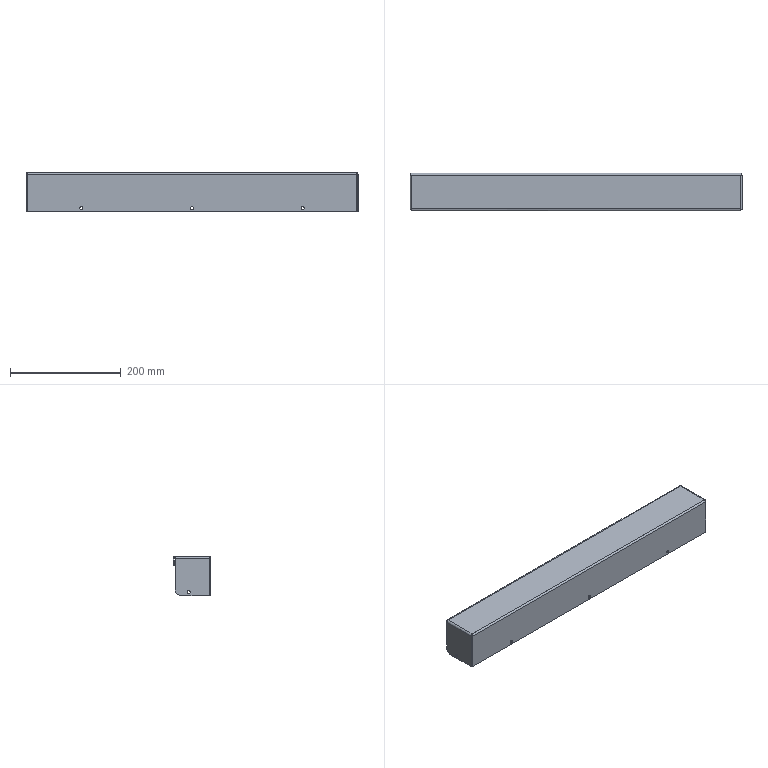Part | NX | 1 solid | 49 faces | box 600 x 68 x 70.5 mm | volume 146489 mm3 | plane 28 | cylinder 17 | spline 4 | commonest cylinder face diameters 5.5 x5 4 x4 7 x4 20 x4
STEP:
#1=CARTESIAN_POINT('',(298.5,30.5,0.));
#2=VERTEX_POINT('',#1);
#3=CARTESIAN_POINT('',(296.5,30.5,0.));
#4=VERTEX_POINT('',#3);
#5=CARTESIAN_POINT('',(298.5,30.5,0.));
#6=DIRECTION('',(1.,0.,0.));
#7=VECTOR('',#6,1000.);
#8=LINE('',#5,#7);
#9=EDGE_CURVE('',#2,#4,#8,.F.);
#10=ORIENTED_EDGE('',*,*,#9,.T.);
#11=CARTESIAN_POINT('',(298.5,30.5,-0.6277));
#12=VERTEX_POINT('',#11);
#13=CARTESIAN_POINT('',(296.5,30.5,-3.5));
#14=DIRECTION('',(0.,-1.,0.));
#15=DIRECTION('',(0.,0.,-1.));
#16=AXIS2_PLACEMENT_3D('',#13,#14,#15);
#17=CIRCLE('',#16,3.5);
#18=EDGE_CURVE('',#4,#12,#17,.F.);
#19=ORIENTED_EDGE('',*,*,#18,.T.);
#20=CARTESIAN_POINT('',(298.5,30.5,-1.5));
#21=DIRECTION('',(0.,0.,1.));
#22=VECTOR('',#21,1000.);
#23=LINE('',#20,#22);
#24=EDGE_CURVE('',#12,#2,#23,.T.);
#25=ORIENTED_EDGE('',*,*,#24,.T.);
#26=EDGE_LOOP('',(#10,#19,#25));
#27=FACE_BOUND('',#26,.T.);
#28=CARTESIAN_POINT('',(296.5,30.5,-1.5));
#29=DIRECTION('',(0.,-1.,0.));
#30=DIRECTION('',(0.,0.,-1.));
#31=AXIS2_PLACEMENT_3D('',#28,#29,#30);
#32=PLANE('',#31);
#33=ADVANCED_FACE('',(#27),#32,.T.);
#34=CARTESIAN_POINT('',(-298.5,30.5,-0.6277));
#35=VERTEX_POINT('',#34);
#36=CARTESIAN_POINT('',(-298.5,30.5,0.));
#37=VERTEX_POINT('',#36);
#38=CARTESIAN_POINT('',(-298.5,30.5,-1.5));
#39=DIRECTION('',(0.,0.,1.));
#40=VECTOR('',#39,1000.);
#41=LINE('',#38,#40);
#42=EDGE_CURVE('',#35,#37,#41,.T.);
#43=ORIENTED_EDGE('',*,*,#42,.F.);
#44=CARTESIAN_POINT('',(-296.5,30.5,0.));
#45=VERTEX_POINT('',#44);
#46=CARTESIAN_POINT('',(-296.5,30.5,-3.5));
#47=DIRECTION('',(0.,1.,0.));
#48=DIRECTION('',(0.,0.,1.));
#49=AXIS2_PLACEMENT_3D('',#46,#47,#48);
#50=CIRCLE('',#49,3.5);
#51=EDGE_CURVE('',#35,#45,#50,.T.);
#52=ORIENTED_EDGE('',*,*,#51,.T.);
#53=CARTESIAN_POINT('',(298.5,30.5,0.));
#54=DIRECTION('',(1.,0.,0.));
#55=VECTOR('',#54,1000.);
#56=LINE('',#53,#55);
#57=EDGE_CURVE('',#37,#45,#56,.T.);
#58=ORIENTED_EDGE('',*,*,#57,.F.);
#59=EDGE_LOOP('',(#43,#52,#58));
#60=FACE_BOUND('',#59,.T.);
#61=CARTESIAN_POINT('',(-298.5,30.5,-1.5));
#62=DIRECTION('',(0.,-1.,0.));
#63=DIRECTION('',(1.,0.,0.));
#64=AXIS2_PLACEMENT_3D('',#61,#62,#63);
#65=PLANE('',#64);
#66=ADVANCED_FACE('',(#60),#65,.T.);
#67=CARTESIAN_POINT('',(296.5,-30.5,-1.5));
#68=VERTEX_POINT('',#67);
#69=CARTESIAN_POINT('',(296.5,30.5,-1.5));
#70=VERTEX_POINT('',#69);
#71=CARTESIAN_POINT('',(296.5,-31.793,-1.5));
#72=DIRECTION('',(0.,-1.,0.));
#73=VECTOR('',#72,1000.);
#74=LINE('',#71,#73);
#75=EDGE_CURVE('',#68,#70,#74,.F.);
#76=ORIENTED_EDGE('',*,*,#75,.F.);
#77=CARTESIAN_POINT('',(-296.5,-30.5,-1.5));
#78=VERTEX_POINT('',#77);
#79=CARTESIAN_POINT('',(-297.793,-30.5,-1.5));
#80=DIRECTION('',(-1.,0.,0.));
#81=VECTOR('',#80,1000.);
#82=LINE('',#79,#81);
#83=EDGE_CURVE('',#78,#68,#82,.F.);
#84=ORIENTED_EDGE('',*,*,#83,.F.);
#85=CARTESIAN_POINT('',(-296.5,30.5,-1.5));
#86=VERTEX_POINT('',#85);
#87=CARTESIAN_POINT('',(-296.5,30.5,-1.5));
#88=DIRECTION('',(0.,1.,0.));
#89=VECTOR('',#88,1000.);
#90=LINE('',#87,#89);
#91=EDGE_CURVE('',#86,#78,#90,.F.);
#92=ORIENTED_EDGE('',*,*,#91,.F.);
#93=CARTESIAN_POINT('',(298.5,30.5,-1.5));
#94=DIRECTION('',(1.,0.,0.));
#95=VECTOR('',#94,1000.);
#96=LINE('',#93,#95);
#97=EDGE_CURVE('',#70,#86,#96,.F.);
#98=ORIENTED_EDGE('',*,*,#97,.F.);
#99=EDGE_LOOP('',(#76,#84,#92,#98));
#100=FACE_BOUND('',#99,.T.);
#101=CARTESIAN_POINT('',(0.,0.,-1.5));
#102=DIRECTION('',(0.,0.,1.));
#103=DIRECTION('',(1.,0.,0.));
#104=AXIS2_PLACEMENT_3D('',#101,#102,#103);
#105=PLANE('',#104);
#106=ADVANCED_FACE('',(#100),#105,.F.);
#107=CARTESIAN_POINT('',(-296.5,-30.5,0.));
#108=VERTEX_POINT('',#107);
#109=CARTESIAN_POINT('',(296.5,-30.5,0.));
#110=VERTEX_POINT('',#109);
#111=CARTESIAN_POINT('',(-297.793,-30.5,0.));
#112=DIRECTION('',(-1.,0.,0.));
#113=VECTOR('',#112,1000.);
#114=LINE('',#111,#113);
#115=EDGE_CURVE('',#108,#110,#114,.F.);
#116=ORIENTED_EDGE('',*,*,#115,.T.);
#117=CARTESIAN_POINT('',(296.5,-31.793,0.));
#118=DIRECTION('',(0.,-1.,0.));
#119=VECTOR('',#118,1000.);
#120=LINE('',#117,#119);
#121=EDGE_CURVE('',#110,#4,#120,.F.);
#122=ORIENTED_EDGE('',*,*,#121,.T.);
#123=CARTESIAN_POINT('',(298.5,30.5,0.));
#124=DIRECTION('',(1.,0.,0.));
#125=VECTOR('',#124,1000.);
#126=LINE('',#123,#125);
#127=EDGE_CURVE('',#4,#45,#126,.F.);
#128=ORIENTED_EDGE('',*,*,#127,.T.);
#129=CARTESIAN_POINT('',(-296.5,30.5,0.));
#130=DIRECTION('',(0.,1.,0.));
#131=VECTOR('',#130,1000.);
#132=LINE('',#129,#131);
#133=EDGE_CURVE('',#45,#108,#132,.F.);
#134=ORIENTED_EDGE('',*,*,#133,.T.);
#135=EDGE_LOOP('',(#116,#122,#128,#134));
#136=FACE_BOUND('',#135,.T.);
#137=CARTESIAN_POINT('',(0.,0.,0.));
#138=DIRECTION('',(0.,0.,1.));
#139=DIRECTION('',(1.,0.,0.));
#140=AXIS2_PLACEMENT_3D('',#137,#138,#139);
#141=PLANE('',#140);
#142=ADVANCED_FACE('',(#136),#141,.T.);
#143=CARTESIAN_POINT('',(-298.5,32.5,-3.5));
#144=VERTEX_POINT('',#143);
#145=CARTESIAN_POINT('',(-298.5,34.,-3.5));
#146=VERTEX_POINT('',#145);
#147=CARTESIAN_POINT('',(-298.5,32.5,-3.5));
#148=DIRECTION('',(0.,1.,0.));
#149=VECTOR('',#148,1000.);
#150=LINE('',#147,#149);
#151=EDGE_CURVE('',#144,#146,#150,.T.);
#152=ORIENTED_EDGE('',*,*,#151,.F.);
#153=CARTESIAN_POINT('',(-298.5,30.5,-1.5));
#154=VERTEX_POINT('',#153);
#155=CARTESIAN_POINT('',(-298.5,30.5,-3.5));
#156=DIRECTION('',(1.,0.,0.));
#157=DIRECTION('',(0.,0.,-1.));
#158=AXIS2_PLACEMENT_3D('',#155,#156,#157);
#159=CIRCLE('',#158,2.);
#160=EDGE_CURVE('',#154,#144,#159,.F.);
#161=ORIENTED_EDGE('',*,*,#160,.F.);
#162=CARTESIAN_POINT('',(-298.5,30.5,-1.5));
#163=DIRECTION('',(0.,0.,1.));
#164=VECTOR('',#163,1000.);
#165=LINE('',#162,#164);
#166=EDGE_CURVE('',#154,#35,#165,.T.);
#167=ORIENTED_EDGE('',*,*,#166,.T.);
#168=ORIENTED_EDGE('',*,*,#42,.T.);
#169=CARTESIAN_POINT('',(-298.5,30.5,-3.5));
#170=DIRECTION('',(1.,0.,0.));
#171=DIRECTION('',(0.,0.,-1.));
#172=AXIS2_PLACEMENT_3D('',#169,#170,#171);
#173=CIRCLE('',#172,3.5);
#174=EDGE_CURVE('',#37,#146,#173,.F.);
#175=ORIENTED_EDGE('',*,*,#174,.T.);
#176=EDGE_LOOP('',(#152,#161,#167,#168,#175));
#177=FACE_BOUND('',#176,.T.);
#178=CARTESIAN_POINT('',(-298.5,30.5,-3.5));
#179=DIRECTION('',(-1.,0.,0.));
#180=DIRECTION('',(0.,0.,1.));
#181=AXIS2_PLACEMENT_3D('',#178,#179,#180);
#182=PLANE('',#181);
#183=ADVANCED_FACE('',(#177),#182,.T.);
#184=CARTESIAN_POINT('',(298.5,32.5,-3.5));
#185=VERTEX_POINT('',#184);
#186=CARTESIAN_POINT('',(298.5,30.5,-1.5));
#187=VERTEX_POINT('',#186);
#188=CARTESIAN_POINT('',(298.5,30.5,-3.5));
#189=DIRECTION('',(1.,0.,0.));
#190=DIRECTION('',(0.,0.,-1.));
#191=AXIS2_PLACEMENT_3D('',#188,#189,#190);
#192=CIRCLE('',#191,2.);
#193=EDGE_CURVE('',#185,#187,#192,.T.);
#194=ORIENTED_EDGE('',*,*,#193,.F.);
#195=CARTESIAN_POINT('',(298.5,34.,-3.5));
#196=VERTEX_POINT('',#195);
#197=CARTESIAN_POINT('',(298.5,32.5,-3.5));
#198=DIRECTION('',(0.,1.,0.));
#199=VECTOR('',#198,1000.);
#200=LINE('',#197,#199);
#201=EDGE_CURVE('',#185,#196,#200,.T.);
#202=ORIENTED_EDGE('',*,*,#201,.T.);
#203=CARTESIAN_POINT('',(298.5,30.5,-3.5));
#204=DIRECTION('',(1.,0.,0.));
#205=DIRECTION('',(0.,0.,-1.));
#206=AXIS2_PLACEMENT_3D('',#203,#204,#205);
#207=CIRCLE('',#206,3.5);
#208=EDGE_CURVE('',#196,#2,#207,.T.);
#209=ORIENTED_EDGE('',*,*,#208,.T.);
#210=ORIENTED_EDGE('',*,*,#24,.F.);
#211=CARTESIAN_POINT('',(298.5,30.5,-1.5));
#212=DIRECTION('',(0.,0.,1.));
#213=VECTOR('',#212,1000.);
#214=LINE('',#211,#213);
#215=EDGE_CURVE('',#187,#12,#214,.T.);
#216=ORIENTED_EDGE('',*,*,#215,.F.);
#217=EDGE_LOOP('',(#194,#202,#209,#210,#216));
#218=FACE_BOUND('',#217,.T.);
#219=CARTESIAN_POINT('',(298.5,30.5,-3.5));
#220=DIRECTION('',(-1.,0.,0.));
#221=DIRECTION('',(0.,0.,1.));
#222=AXIS2_PLACEMENT_3D('',#219,#220,#221);
#223=PLANE('',#222);
#224=ADVANCED_FACE('',(#218),#223,.F.);
#225=ORIENTED_EDGE('',*,*,#9,.F.);
#226=ORIENTED_EDGE('',*,*,#208,.F.);
#227=CARTESIAN_POINT('',(0.,34.,-3.5));
#228=DIRECTION('',(-1.,0.,0.));
#229=VECTOR('',#228,1000.);
#230=LINE('',#227,#229);
#231=EDGE_CURVE('',#196,#146,#230,.T.);
#232=ORIENTED_EDGE('',*,*,#231,.T.);
#233=ORIENTED_EDGE('',*,*,#174,.F.);
#234=ORIENTED_EDGE('',*,*,#57,.T.);
#235=ORIENTED_EDGE('',*,*,#127,.F.);
#236=EDGE_LOOP('',(#225,#226,#232,#233,#234,#235));
#237=FACE_BOUND('',#236,.T.);
#238=CARTESIAN_POINT('',(298.5,30.5,-3.5));
#239=DIRECTION('',(1.,0.,0.));
#240=DIRECTION('',(0.,1.,0.));
#241=AXIS2_PLACEMENT_3D('',#238,#239,#240);
#242=CYLINDRICAL_SURFACE('',#241,3.5);
#243=ADVANCED_FACE('',(#237),#242,.T.);
#244=CARTESIAN_POINT('',(298.5,30.5,-1.5));
#245=DIRECTION('',(1.,0.,0.));
#246=VECTOR('',#245,1000.);
#247=LINE('',#244,#246);
#248=EDGE_CURVE('',#187,#70,#247,.F.);
#249=ORIENTED_EDGE('',*,*,#248,.T.);
#250=ORIENTED_EDGE('',*,*,#97,.T.);
#251=CARTESIAN_POINT('',(-298.5,30.5,-1.5));
#252=DIRECTION('',(1.,0.,0.));
#253=VECTOR('',#252,1000.);
#254=LINE('',#251,#253);
#255=EDGE_CURVE('',#154,#86,#254,.T.);
#256=ORIENTED_EDGE('',*,*,#255,.F.);
#257=ORIENTED_EDGE('',*,*,#160,.T.);
#258=CARTESIAN_POINT('',(-298.5,32.5,-3.5));
#259=DIRECTION('',(1.,0.,0.));
#260=VECTOR('',#259,1000.);
#261=LINE('',#258,#260);
#262=EDGE_CURVE('',#144,#185,#261,.T.);
#263=ORIENTED_EDGE('',*,*,#262,.T.);
#264=ORIENTED_EDGE('',*,*,#193,.T.);
#265=EDGE_LOOP('',(#249,#250,#256,#257,#263,#264));
#266=FACE_BOUND('',#265,.T.);
#267=CARTESIAN_POINT('',(298.5,30.5,-3.5));
#268=DIRECTION('',(1.,0.,0.));
#269=DIRECTION('',(0.,1.,0.));
#270=AXIS2_PLACEMENT_3D('',#267,#268,#269);
#271=CYLINDRICAL_SURFACE('',#270,2.);
#272=ADVANCED_FACE('',(#266),#271,.F.);
#273=CARTESIAN_POINT('',(298.5,32.5,-6.5));
#274=VERTEX_POINT('',#273);
#275=CARTESIAN_POINT('',(298.5,32.5,-16.5));
#276=DIRECTION('',(0.,0.,-1.));
#277=VECTOR('',#276,1000.);
#278=LINE('',#275,#277);
#279=EDGE_CURVE('',#185,#274,#278,.T.);
#280=ORIENTED_EDGE('',*,*,#279,.T.);
#281=CARTESIAN_POINT('',(298.5,34.,-6.5));
#282=VERTEX_POINT('',#281);
#283=CARTESIAN_POINT('',(298.5,34.,-6.5));
#284=DIRECTION('',(0.,-1.,0.));
#285=VECTOR('',#284,1000.);
#286=LINE('',#283,#285);
#287=EDGE_CURVE('',#274,#282,#286,.F.);
#288=ORIENTED_EDGE('',*,*,#287,.T.);
#289=CARTESIAN_POINT('',(298.5,34.,-16.5));
#290=DIRECTION('',(0.,0.,-1.));
#291=VECTOR('',#290,1000.);
#292=LINE('',#289,#291);
#293=EDGE_CURVE('',#196,#282,#292,.T.);
#294=ORIENTED_EDGE('',*,*,#293,.F.);
#295=ORIENTED_EDGE('',*,*,#201,.F.);
#296=EDGE_LOOP('',(#280,#288,#294,#295));
#297=FACE_BOUND('',#296,.T.);
#298=CARTESIAN_POINT('',(298.5,34.,-16.5));
#299=DIRECTION('',(-1.,0.,0.));
#300=DIRECTION('',(0.,0.,1.));
#301=AXIS2_PLACEMENT_3D('',#298,#299,#300);
#302=PLANE('',#301);
#303=ADVANCED_FACE('',(#297),#302,.F.);
#304=CARTESIAN_POINT('',(-298.5,34.,-6.5));
#305=VERTEX_POINT('',#304);
#306=CARTESIAN_POINT('',(-298.5,34.,-1.5));
#307=DIRECTION('',(0.,0.,1.));
#308=VECTOR('',#307,1000.);
#309=LINE('',#306,#308);
#310=EDGE_CURVE('',#305,#146,#309,.T.);
#311=ORIENTED_EDGE('',*,*,#310,.F.);
#312=CARTESIAN_POINT('',(-298.5,32.5,-6.5));
#313=VERTEX_POINT('',#312);
#314=CARTESIAN_POINT('',(-298.5,34.,-6.5));
#315=DIRECTION('',(0.,-1.,0.));
#316=VECTOR('',#315,1000.);
#317=LINE('',#314,#316);
#318=EDGE_CURVE('',#305,#313,#317,.T.);
#319=ORIENTED_EDGE('',*,*,#318,.T.);
#320=CARTESIAN_POINT('',(-298.5,32.5,-1.5));
#321=DIRECTION('',(0.,0.,1.));
#322=VECTOR('',#321,1000.);
#323=LINE('',#320,#322);
#324=EDGE_CURVE('',#313,#144,#323,.T.);
#325=ORIENTED_EDGE('',*,*,#324,.T.);
#326=ORIENTED_EDGE('',*,*,#151,.T.);
#327=EDGE_LOOP('',(#311,#319,#325,#326));
#328=FACE_BOUND('',#327,.T.);
#329=CARTESIAN_POINT('',(-298.5,34.,-1.5));
#330=DIRECTION('',(1.,0.,0.));
#331=DIRECTION('',(0.,0.,-1.));
#332=AXIS2_PLACEMENT_3D('',#329,#330,#331);
#333=PLANE('',#332);
#334=ADVANCED_FACE('',(#328),#333,.F.);
#335=ORIENTED_EDGE('',*,*,#293,.T.);
#336=CARTESIAN_POINT('',(288.5,34.,-16.5));
#337=VERTEX_POINT('',#336);
#338=CARTESIAN_POINT('',(288.5,34.,-6.5));
#339=DIRECTION('',(0.,-1.,0.));
#340=DIRECTION('',(0.,0.,-1.));
#341=AXIS2_PLACEMENT_3D('',#338,#339,#340);
#342=CIRCLE('',#341,10.);
#343=EDGE_CURVE('',#282,#337,#342,.F.);
#344=ORIENTED_EDGE('',*,*,#343,.T.);
#345=CARTESIAN_POINT('',(-288.5,34.,-16.5));
#346=VERTEX_POINT('',#345);
#347=CARTESIAN_POINT('',(-298.5,34.,-16.5));
#348=DIRECTION('',(-1.,0.,0.));
#349=VECTOR('',#348,1000.);
#350=LINE('',#347,#349);
#351=EDGE_CURVE('',#337,#346,#350,.T.);
#352=ORIENTED_EDGE('',*,*,#351,.T.);
#353=CARTESIAN_POINT('',(-288.5,34.,-6.5));
#354=DIRECTION('',(0.,-1.,0.));
#355=DIRECTION('',(0.,0.,-1.));
#356=AXIS2_PLACEMENT_3D('',#353,#354,#355);
#357=CIRCLE('',#356,10.);
#358=EDGE_CURVE('',#346,#305,#357,.F.);
#359=ORIENTED_EDGE('',*,*,#358,.T.);
#360=ORIENTED_EDGE('',*,*,#310,.T.);
#361=ORIENTED_EDGE('',*,*,#231,.F.);
#362=EDGE_LOOP('',(#335,#344,#352,#359,#360,#361));
#363=FACE_BOUND('',#362,.T.);
#364=CARTESIAN_POINT('',(0.,34.,0.));
#365=DIRECTION('',(0.,-1.,0.));
#366=DIRECTION('',(0.,0.,-1.));
#367=AXIS2_PLACEMENT_3D('',#364,#365,#366);
#368=PLANE('',#367);
#369=ADVANCED_FACE('',(#363),#368,.F.);
#370=CARTESIAN_POINT('',(288.5,32.5,-16.5));
#371=VERTEX_POINT('',#370);
#372=CARTESIAN_POINT('',(-288.5,32.5,-16.5));
#373=VERTEX_POINT('',#372);
#374=CARTESIAN_POINT('',(-298.5,32.5,-16.5));
#375=DIRECTION('',(-1.,0.,0.));
#376=VECTOR('',#375,1000.);
#377=LINE('',#374,#376);
#378=EDGE_CURVE('',#371,#373,#377,.T.);
#379=ORIENTED_EDGE('',*,*,#378,.F.);
#380=CARTESIAN_POINT('',(288.5,32.5,-6.5));
#381=DIRECTION('',(0.,-1.,0.));
#382=DIRECTION('',(0.,0.,-1.));
#383=AXIS2_PLACEMENT_3D('',#380,#381,#382);
#384=CIRCLE('',#383,10.);
#385=EDGE_CURVE('',#371,#274,#384,.T.);
#386=ORIENTED_EDGE('',*,*,#385,.T.);
#387=ORIENTED_EDGE('',*,*,#279,.F.);
#388=ORIENTED_EDGE('',*,*,#262,.F.);
#389=ORIENTED_EDGE('',*,*,#324,.F.);
#390=CARTESIAN_POINT('',(-288.5,32.5,-6.5));
#391=DIRECTION('',(0.,-1.,0.));
#392=DIRECTION('',(0.,0.,-1.));
#393=AXIS2_PLACEMENT_3D('',#390,#391,#392);
#394=CIRCLE('',#393,10.);
#395=EDGE_CURVE('',#313,#373,#394,.T.);
#396=ORIENTED_EDGE('',*,*,#395,.T.);
#397=EDGE_LOOP('',(#379,#386,#387,#388,#389,#396));
#398=FACE_BOUND('',#397,.T.);
#399=CARTESIAN_POINT('',(0.,32.5,0.));
#400=DIRECTION('',(0.,-1.,0.));
#401=DIRECTION('',(0.,0.,-1.));
#402=AXIS2_PLACEMENT_3D('',#399,#400,#401);
#403=PLANE('',#402);
#404=ADVANCED_FACE('',(#398),#403,.T.);
#405=ORIENTED_EDGE('',*,*,#351,.F.);
#406=CARTESIAN_POINT('',(288.5,34.,-16.5));
#407=DIRECTION('',(0.,-1.,0.));
#408=VECTOR('',#407,1000.);
#409=LINE('',#406,#408);
#410=EDGE_CURVE('',#337,#371,#409,.T.);
#411=ORIENTED_EDGE('',*,*,#410,.T.);
#412=ORIENTED_EDGE('',*,*,#378,.T.);
#413=CARTESIAN_POINT('',(-288.5,34.,-16.5));
#414=DIRECTION('',(0.,-1.,0.));
#415=VECTOR('',#414,1000.);
#416=LINE('',#413,#415);
#417=EDGE_CURVE('',#373,#346,#416,.F.);
#418=ORIENTED_EDGE('',*,*,#417,.T.);
#419=EDGE_LOOP('',(#405,#411,#412,#418));
#420=FACE_BOUND('',#419,.T.);
#421=CARTESIAN_POINT('',(-298.5,34.,-16.5));
#422=DIRECTION('',(0.,0.,1.));
#423=DIRECTION('',(0.,-1.,0.));
#424=AXIS2_PLACEMENT_3D('',#421,#422,#423);
#425=PLANE('',#424);
#426=ADVANCED_FACE('',(#420),#425,.F.);
#427=ORIENTED_EDGE('',*,*,#166,.F.);
#428=ORIENTED_EDGE('',*,*,#255,.T.);
#429=CARTESIAN_POINT('',(-298.5,30.5,-3.5));
#430=VERTEX_POINT('',#429);
#431=CARTESIAN_POINT('',(-296.5,30.5,-3.5));
#432=DIRECTION('',(0.,1.,0.));
#433=DIRECTION('',(0.,0.,1.));
#434=AXIS2_PLACEMENT_3D('',#431,#432,#433);
#435=CIRCLE('',#434,2.);
#436=EDGE_CURVE('',#430,#86,#435,.T.);
#437=ORIENTED_EDGE('',*,*,#436,.F.);
#438=CARTESIAN_POINT('',(-300.,30.5,-3.5));
#439=VERTEX_POINT('',#438);
#440=CARTESIAN_POINT('',(-298.5,30.5,-3.5));
#441=DIRECTION('',(-1.,0.,0.));
#442=VECTOR('',#441,1000.);
#443=LINE('',#440,#442);
#444=EDGE_CURVE('',#430,#439,#443,.T.);
#445=ORIENTED_EDGE('',*,*,#444,.T.);
#446=CARTESIAN_POINT('',(-296.5,30.5,-3.5));
#447=DIRECTION('',(0.,1.,0.));
#448=DIRECTION('',(0.,0.,1.));
#449=AXIS2_PLACEMENT_3D('',#446,#447,#448);
#450=CIRCLE('',#449,3.5);
#451=EDGE_CURVE('',#439,#35,#450,.T.);
#452=ORIENTED_EDGE('',*,*,#451,.T.);
#453=EDGE_LOOP('',(#427,#428,#437,#445,#452));
#454=FACE_BOUND('',#453,.T.);
#455=CARTESIAN_POINT('',(-296.5,30.5,-3.5));
#456=DIRECTION('',(0.,-1.,0.));
#457=DIRECTION('',(0.,0.,-1.));
#458=AXIS2_PLACEMENT_3D('',#455,#456,#457);
#459=PLANE('',#458);
#460=ADVANCED_FACE('',(#454),#459,.F.);
#461=CARTESIAN_POINT('',(-300.,-31.793,-3.5));
#462=VERTEX_POINT('',#461);
#463=CARTESIAN_POINT('',(-298.5,-31.793,-3.5));
#464=VERTEX_POINT('',#463);
#465=CARTESIAN_POINT('',(-298.5,-31.793,-3.5));
#466=DIRECTION('',(1.,0.,0.));
#467=VECTOR('',#466,1000.);
#468=LINE('',#465,#467);
#469=EDGE_CURVE('',#462,#464,#468,.T.);
#470=ORIENTED_EDGE('',*,*,#469,.T.);
#471=CARTESIAN_POINT('',(-296.5,-30.5,-1.5));
#472=CARTESIAN_POINT('',(-297.028,-30.717,-1.5));
#473=CARTESIAN_POINT('',(-298.064,-31.146,-1.935));
#474=CARTESIAN_POINT('',(-298.5,-31.575,-2.972));
#475=CARTESIAN_POINT('',(-298.5,-31.793,-3.5));
#476=B_SPLINE_CURVE_WITH_KNOTS('',3,(#471,#472,#473,#474,#475),.UNSPECIFIED.,.F.,.F.,(4,1,4),(0.,0.00169,0.00338),.UNSPECIFIED.);
#477=EDGE_CURVE('',#78,#464,#476,.T.);
#478=ORIENTED_EDGE('',*,*,#477,.F.);
#479=CARTESIAN_POINT('',(-296.5,-30.5,-1.5));
#480=DIRECTION('',(0.,0.,1.));
#481=VECTOR('',#480,1000.);
#482=LINE('',#479,#481);
#483=EDGE_CURVE('',#78,#108,#482,.T.);
#484=ORIENTED_EDGE('',*,*,#483,.T.);
#485=CARTESIAN_POINT('',(-296.5,-30.5,0.));
#486=CARTESIAN_POINT('',(-297.424,-30.717,0.));
#487=CARTESIAN_POINT('',(-299.236,-31.146,-0.7608));
#488=CARTESIAN_POINT('',(-300.,-31.576,-2.576));
#489=CARTESIAN_POINT('',(-300.,-31.793,-3.5));
#490=B_SPLINE_CURVE_WITH_KNOTS('',3,(#485,#486,#487,#488,#489),.UNSPECIFIED.,.F.,.F.,(4,1,4),(0.,0.002808,0.005617),.UNSPECIFIED.);
#491=EDGE_CURVE('',#108,#462,#490,.T.);
#492=ORIENTED_EDGE('',*,*,#491,.T.);
#493=EDGE_LOOP('',(#470,#478,#484,#492));
#494=FACE_BOUND('',#493,.T.);
#495=CARTESIAN_POINT('',(-296.5,-30.5,0.015));
#496=CARTESIAN_POINT('',(-296.96,-30.608,0.015));
#497=CARTESIAN_POINT('',(-297.42,-30.715,-0.07649));
#498=CARTESIAN_POINT('',(-298.27,-30.931,-0.4286));
#499=CARTESIAN_POINT('',(-298.66,-31.039,-0.6892));
#500=CARTESIAN_POINT('',(-299.311,-31.254,-1.34));
#501=CARTESIAN_POINT('',(-299.571,-31.362,-1.73));
#502=CARTESIAN_POINT('',(-299.924,-31.577,-2.58));
#503=CARTESIAN_POINT('',(-300.015,-31.685,-3.04));
#504=CARTESIAN_POINT('',(-300.015,-31.793,-3.5));
#505=CARTESIAN_POINT('',(-296.5,-30.5,0.));
#506=CARTESIAN_POINT('',(-296.958,-30.608,0.));
#507=CARTESIAN_POINT('',(-297.416,-30.715,-0.0911));
#508=CARTESIAN_POINT('',(-298.263,-30.931,-0.4417));
#509=CARTESIAN_POINT('',(-298.651,-31.039,-0.7012));
#510=CARTESIAN_POINT('',(-299.299,-31.254,-1.349));
#511=CARTESIAN_POINT('',(-299.558,-31.362,-1.737));
#512=CARTESIAN_POINT('',(-299.909,-31.577,-2.584));
#513=CARTESIAN_POINT('',(-300.,-31.685,-3.042));
#514=CARTESIAN_POINT('',(-300.,-31.793,-3.5));
#515=CARTESIAN_POINT('',(-296.5,-30.5,-1.5));
#516=CARTESIAN_POINT('',(-296.762,-30.608,-1.5));
#517=CARTESIAN_POINT('',(-297.023,-30.715,-1.552));
#518=CARTESIAN_POINT('',(-297.507,-30.931,-1.752));
#519=CARTESIAN_POINT('',(-297.729,-31.039,-1.901));
#520=CARTESIAN_POINT('',(-298.099,-31.254,-2.271));
#521=CARTESIAN_POINT('',(-298.248,-31.362,-2.493));
#522=CARTESIAN_POINT('',(-298.448,-31.577,-2.977));
#523=CARTESIAN_POINT('',(-298.5,-31.685,-3.238));
#524=CARTESIAN_POINT('',(-298.5,-31.793,-3.5));
#525=CARTESIAN_POINT('',(-296.5,-30.5,-1.515));
#526=CARTESIAN_POINT('',(-296.76,-30.608,-1.515));
#527=CARTESIAN_POINT('',(-297.02,-30.715,-1.567));
#528=CARTESIAN_POINT('',(-297.5,-30.931,-1.766));
#529=CARTESIAN_POINT('',(-297.72,-31.039,-1.913));
#530=CARTESIAN_POINT('',(-298.087,-31.254,-2.28));
#531=CARTESIAN_POINT('',(-298.234,-31.362,-2.5));
#532=CARTESIAN_POINT('',(-298.433,-31.577,-2.98));
#533=CARTESIAN_POINT('',(-298.485,-31.685,-3.24));
#534=CARTESIAN_POINT('',(-298.485,-31.793,-3.5));
#535=B_SPLINE_SURFACE_WITH_KNOTS('',1,3,((#495,#496,#497,#498,#499,#500,#501,#502,#503,#504),(#505,#506,#507,#508,#509,#510,#511,#512,#513,#514),(#515,#516,#517,#518,#519,#520,#521,#522,#523,#524),(#525,#526,#527,#528,#529,#530,#531,#532,#533,#534)),.RULED_SURF.,.F.,.F.,.F.,(2,1,1,2),(4,2,2,2,4),(-0.01,0.,1.,1.01),(0.,0.25,0.5,0.75,1.),.UNSPECIFIED.);
#536=ADVANCED_FACE('',(#494),#535,.F.);
#537=ORIENTED_EDGE('',*,*,#133,.F.);
#538=ORIENTED_EDGE('',*,*,#51,.F.);
#539=ORIENTED_EDGE('',*,*,#451,.F.);
#540=CARTESIAN_POINT('',(-300.,0.,-3.5));
#541=DIRECTION('',(0.,-1.,0.));
#542=VECTOR('',#541,1000.);
#543=LINE('',#540,#542);
#544=EDGE_CURVE('',#439,#462,#543,.T.);
#545=ORIENTED_EDGE('',*,*,#544,.T.);
#546=ORIENTED_EDGE('',*,*,#491,.F.);
#547=EDGE_LOOP('',(#537,#538,#539,#545,#546));
#548=FACE_BOUND('',#547,.T.);
#549=CARTESIAN_POINT('',(-296.5,30.5,-3.5));
#550=DIRECTION('',(0.,1.,0.));
#551=DIRECTION('',(-1.,0.,0.));
#552=AXIS2_PLACEMENT_3D('',#549,#550,#551);
#553=CYLINDRICAL_SURFACE('',#552,3.5);
#554=ADVANCED_FACE('',(#548),#553,.T.);
#555=ORIENTED_EDGE('',*,*,#91,.T.);
#556=ORIENTED_EDGE('',*,*,#477,.T.);
#557=CARTESIAN_POINT('',(-298.5,-32.5,-3.5));
#558=DIRECTION('',(0.,1.,0.));
#559=VECTOR('',#558,1000.);
#560=LINE('',#557,#559);
#561=EDGE_CURVE('',#464,#430,#560,.T.);
#562=ORIENTED_EDGE('',*,*,#561,.T.);
#563=ORIENTED_EDGE('',*,*,#436,.T.);
#564=EDGE_LOOP('',(#555,#556,#562,#563));
#565=FACE_BOUND('',#564,.T.);
#566=CARTESIAN_POINT('',(-296.5,30.5,-3.5));
#567=DIRECTION('',(0.,1.,0.));
#568=DIRECTION('',(-1.,0.,0.));
#569=AXIS2_PLACEMENT_3D('',#566,#567,#568);
#570=CYLINDRICAL_SURFACE('',#569,2.);
#571=ADVANCED_FACE('',(#565),#570,.F.);
#572=CARTESIAN_POINT('',(-300.,-31.793,-70.5));
#573=VERTEX_POINT('',#572);
#574=CARTESIAN_POINT('',(-300.,-31.793,0.));
#575=DIRECTION('',(0.,0.,-1.));
#576=VECTOR('',#575,1000.);
#577=LINE('',#574,#576);
#578=EDGE_CURVE('',#462,#573,#577,.T.);
#579=ORIENTED_EDGE('',*,*,#578,.T.);
#580=CARTESIAN_POINT('',(-298.5,-31.793,-70.5));
#581=VERTEX_POINT('',#580);
#582=CARTESIAN_POINT('',(-300.,-31.793,-70.5));
#583=DIRECTION('',(1.,0.,0.));
#584=VECTOR('',#583,1000.);
#585=LINE('',#582,#584);
#586=EDGE_CURVE('',#573,#581,#585,.T.);
#587=ORIENTED_EDGE('',*,*,#586,.T.);
#588=CARTESIAN_POINT('',(-298.5,-31.793,-1.5));
#589=DIRECTION('',(0.,0.,-1.));
#590=VECTOR('',#589,1000.);
#591=LINE('',#588,#590);
#592=EDGE_CURVE('',#464,#581,#591,.T.);
#593=ORIENTED_EDGE('',*,*,#592,.F.);
#594=ORIENTED_EDGE('',*,*,#469,.F.);
#595=EDGE_LOOP('',(#579,#587,#593,#594));
#596=FACE_BOUND('',#595,.T.);
#597=CARTESIAN_POINT('',(-298.5,-31.793,-1.5));
#598=DIRECTION('',(0.,-1.,0.));
#599=DIRECTION('',(0.,0.,-1.));
#600=AXIS2_PLACEMENT_3D('',#597,#598,#599);
#601=PLANE('',#600);
#602=ADVANCED_FACE('',(#596),#601,.T.);
#603=CARTESIAN_POINT('',(-300.,6.,-61.75));
#604=VERTEX_POINT('',#603);
#605=CARTESIAN_POINT('',(-300.,6.,-64.5));
#606=DIRECTION('',(-1.,0.,0.));
#607=DIRECTION('',(0.,0.,1.));
#608=AXIS2_PLACEMENT_3D('',#605,#606,#607);
#609=CIRCLE('',#608,2.75);
#610=EDGE_CURVE('',#604,#604,#609,.T.);
#611=ORIENTED_EDGE('',*,*,#610,.F.);
#612=EDGE_LOOP('',(#611));
#613=FACE_BOUND('',#612,.T.);
#614=CARTESIAN_POINT('',(-300.,30.5,-60.5));
#615=VERTEX_POINT('',#614);
#616=CARTESIAN_POINT('',(-300.,30.5,-70.5));
#617=DIRECTION('',(0.,0.,-1.));
#618=VECTOR('',#617,1000.);
#619=LINE('',#616,#618);
#620=EDGE_CURVE('',#439,#615,#619,.T.);
#621=ORIENTED_EDGE('',*,*,#620,.T.);
#622=CARTESIAN_POINT('',(-300.,20.5,-70.5));
#623=VERTEX_POINT('',#622);
#624=CARTESIAN_POINT('',(-300.,20.5,-60.5));
#625=DIRECTION('',(1.,0.,0.));
#626=DIRECTION('',(0.,0.,-1.));
#627=AXIS2_PLACEMENT_3D('',#624,#625,#626);
#628=CIRCLE('',#627,10.);
#629=EDGE_CURVE('',#615,#623,#628,.F.);
#630=ORIENTED_EDGE('',*,*,#629,.T.);
#631=CARTESIAN_POINT('',(-300.,-32.5,-70.5));
#632=DIRECTION('',(0.,-1.,0.));
#633=VECTOR('',#632,1000.);
#634=LINE('',#631,#633);
#635=EDGE_CURVE('',#623,#573,#634,.T.);
#636=ORIENTED_EDGE('',*,*,#635,.T.);
#637=ORIENTED_EDGE('',*,*,#578,.F.);
#638=ORIENTED_EDGE('',*,*,#544,.F.);
#639=EDGE_LOOP('',(#621,#630,#636,#637,#638));
#640=FACE_BOUND('',#639,.T.);
#641=CARTESIAN_POINT('',(-300.,0.,0.));
#642=DIRECTION('',(1.,0.,0.));
#643=DIRECTION('',(0.,0.,-1.));
#644=AXIS2_PLACEMENT_3D('',#641,#642,#643);
#645=PLANE('',#644);
#646=ADVANCED_FACE('',(#613,#640),#645,.F.);
#647=CARTESIAN_POINT('',(-298.5,6.,-67.25));
#648=VERTEX_POINT('',#647);
#649=CARTESIAN_POINT('',(-298.5,6.,-64.5));
#650=DIRECTION('',(1.,0.,0.));
#651=DIRECTION('',(0.,0.,-1.));
#652=AXIS2_PLACEMENT_3D('',#649,#650,#651);
#653=CIRCLE('',#652,2.75);
#654=EDGE_CURVE('',#648,#648,#653,.T.);
#655=ORIENTED_EDGE('',*,*,#654,.F.);
#656=EDGE_LOOP('',(#655));
#657=FACE_BOUND('',#656,.T.);
#658=CARTESIAN_POINT('',(-298.5,20.5,-70.5));
#659=VERTEX_POINT('',#658);
#660=CARTESIAN_POINT('',(-298.5,-32.5,-70.5));
#661=DIRECTION('',(0.,-1.,0.));
#662=VECTOR('',#661,1000.);
#663=LINE('',#660,#662);
#664=EDGE_CURVE('',#659,#581,#663,.T.);
#665=ORIENTED_EDGE('',*,*,#664,.F.);
#666=CARTESIAN_POINT('',(-298.5,30.5,-60.5));
#667=VERTEX_POINT('',#666);
#668=CARTESIAN_POINT('',(-298.5,20.5,-60.5));
#669=DIRECTION('',(1.,0.,0.));
#670=DIRECTION('',(0.,0.,-1.));
#671=AXIS2_PLACEMENT_3D('',#668,#669,#670);
#672=CIRCLE('',#671,10.);
#673=EDGE_CURVE('',#659,#667,#672,.T.);
#674=ORIENTED_EDGE('',*,*,#673,.T.);
#675=CARTESIAN_POINT('',(-298.5,30.5,-70.5));
#676=DIRECTION('',(0.,0.,-1.));
#677=VECTOR('',#676,1000.);
#678=LINE('',#675,#677);
#679=EDGE_CURVE('',#430,#667,#678,.T.);
#680=ORIENTED_EDGE('',*,*,#679,.F.);
#681=ORIENTED_EDGE('',*,*,#561,.F.);
#682=ORIENTED_EDGE('',*,*,#592,.T.);
#683=EDGE_LOOP('',(#665,#674,#680,#681,#682));
#684=FACE_BOUND('',#683,.T.);
#685=CARTESIAN_POINT('',(-298.5,0.,0.));
#686=DIRECTION('',(1.,0.,0.));
#687=DIRECTION('',(0.,0.,-1.));
#688=AXIS2_PLACEMENT_3D('',#685,#686,#687);
#689=PLANE('',#688);
#690=ADVANCED_FACE('',(#657,#684),#689,.T.);
#691=ORIENTED_EDGE('',*,*,#635,.F.);
#692=CARTESIAN_POINT('',(-300.,20.5,-70.5));
#693=DIRECTION('',(1.,0.,0.));
#694=VECTOR('',#693,1000.);
#695=LINE('',#692,#694);
#696=EDGE_CURVE('',#623,#659,#695,.T.);
#697=ORIENTED_EDGE('',*,*,#696,.T.);
#698=ORIENTED_EDGE('',*,*,#664,.T.);
#699=ORIENTED_EDGE('',*,*,#586,.F.);
#700=EDGE_LOOP('',(#691,#697,#698,#699));
#701=FACE_BOUND('',#700,.T.);
#702=CARTESIAN_POINT('',(-300.,-32.5,-70.5));
#703=DIRECTION('',(0.,0.,1.));
#704=DIRECTION('',(1.,0.,0.));
#705=AXIS2_PLACEMENT_3D('',#702,#703,#704);
#706=PLANE('',#705);
#707=ADVANCED_FACE('',(#701),#706,.F.);
#708=ORIENTED_EDGE('',*,*,#679,.T.);
#709=CARTESIAN_POINT('',(-300.,30.5,-60.5));
#710=DIRECTION('',(1.,0.,0.));
#711=VECTOR('',#710,1000.);
#712=LINE('',#709,#711);
#713=EDGE_CURVE('',#667,#615,#712,.F.);
#714=ORIENTED_EDGE('',*,*,#713,.T.);
#715=ORIENTED_EDGE('',*,*,#620,.F.);
#716=ORIENTED_EDGE('',*,*,#444,.F.);
#717=EDGE_LOOP('',(#708,#714,#715,#716));
#718=FACE_BOUND('',#717,.T.);
#719=CARTESIAN_POINT('',(-300.,30.5,-70.5));
#720=DIRECTION('',(0.,-1.,0.));
#721=DIRECTION('',(1.,0.,0.));
#722=AXIS2_PLACEMENT_3D('',#719,#720,#721);
#723=PLANE('',#722);
#724=ADVANCED_FACE('',(#718),#723,.F.);
#725=CARTESIAN_POINT('',(297.793,-34.,-3.5));
#726=VERTEX_POINT('',#725);
#727=CARTESIAN_POINT('',(297.793,-32.5,-3.5));
#728=VERTEX_POINT('',#727);
#729=CARTESIAN_POINT('',(297.793,-32.5,-3.5));
#730=DIRECTION('',(0.,1.,0.));
#731=VECTOR('',#730,1000.);
#732=LINE('',#729,#731);
#733=EDGE_CURVE('',#726,#728,#732,.T.);
#734=ORIENTED_EDGE('',*,*,#733,.T.);
#735=CARTESIAN_POINT('',(296.5,-30.5,-1.5));
#736=CARTESIAN_POINT('',(296.717,-31.028,-1.5));
#737=CARTESIAN_POINT('',(297.146,-32.064,-1.935));
#738=CARTESIAN_POINT('',(297.575,-32.5,-2.972));
#739=CARTESIAN_POINT('',(297.793,-32.5,-3.5));
#740=B_SPLINE_CURVE_WITH_KNOTS('',3,(#735,#736,#737,#738,#739),.UNSPECIFIED.,.F.,.F.,(4,1,4),(0.,0.00169,0.00338),.UNSPECIFIED.);
#741=EDGE_CURVE('',#68,#728,#740,.T.);
#742=ORIENTED_EDGE('',*,*,#741,.F.);
#743=CARTESIAN_POINT('',(296.5,-30.5,-1.5));
#744=DIRECTION('',(0.,0.,1.));
#745=VECTOR('',#744,1000.);
#746=LINE('',#743,#745);
#747=EDGE_CURVE('',#68,#110,#746,.T.);
#748=ORIENTED_EDGE('',*,*,#747,.T.);
#749=CARTESIAN_POINT('',(296.5,-30.5,0.));
#750=CARTESIAN_POINT('',(296.717,-31.424,0.));
#751=CARTESIAN_POINT('',(297.146,-33.236,-0.7608));
#752=CARTESIAN_POINT('',(297.576,-34.,-2.576));
#753=CARTESIAN_POINT('',(297.793,-34.,-3.5));
#754=B_SPLINE_CURVE_WITH_KNOTS('',3,(#749,#750,#751,#752,#753),.UNSPECIFIED.,.F.,.F.,(4,1,4),(0.,0.002808,0.005617),.UNSPECIFIED.);
#755=EDGE_CURVE('',#110,#726,#754,.T.);
#756=ORIENTED_EDGE('',*,*,#755,.T.);
#757=EDGE_LOOP('',(#734,#742,#748,#756));
#758=FACE_BOUND('',#757,.T.);
#759=CARTESIAN_POINT('',(296.5,-30.5,0.015));
#760=CARTESIAN_POINT('',(296.608,-30.96,0.015));
#761=CARTESIAN_POINT('',(296.715,-31.42,-0.07649));
#762=CARTESIAN_POINT('',(296.931,-32.27,-0.4286));
#763=CARTESIAN_POINT('',(297.039,-32.66,-0.6892));
#764=CARTESIAN_POINT('',(297.254,-33.311,-1.34));
#765=CARTESIAN_POINT('',(297.362,-33.571,-1.73));
#766=CARTESIAN_POINT('',(297.577,-33.924,-2.58));
#767=CARTESIAN_POINT('',(297.685,-34.015,-3.04));
#768=CARTESIAN_POINT('',(297.793,-34.015,-3.5));
#769=CARTESIAN_POINT('',(296.5,-30.5,0.));
#770=CARTESIAN_POINT('',(296.608,-30.958,0.));
#771=CARTESIAN_POINT('',(296.715,-31.416,-0.0911));
#772=CARTESIAN_POINT('',(296.931,-32.263,-0.4417));
#773=CARTESIAN_POINT('',(297.039,-32.651,-0.7012));
#774=CARTESIAN_POINT('',(297.254,-33.299,-1.349));
#775=CARTESIAN_POINT('',(297.362,-33.558,-1.737));
#776=CARTESIAN_POINT('',(297.577,-33.909,-2.584));
#777=CARTESIAN_POINT('',(297.685,-34.,-3.042));
#778=CARTESIAN_POINT('',(297.793,-34.,-3.5));
#779=CARTESIAN_POINT('',(296.5,-30.5,-1.5));
#780=CARTESIAN_POINT('',(296.608,-30.762,-1.5));
#781=CARTESIAN_POINT('',(296.715,-31.023,-1.552));
#782=CARTESIAN_POINT('',(296.931,-31.507,-1.752));
#783=CARTESIAN_POINT('',(297.039,-31.729,-1.901));
#784=CARTESIAN_POINT('',(297.254,-32.099,-2.271));
#785=CARTESIAN_POINT('',(297.362,-32.248,-2.493));
#786=CARTESIAN_POINT('',(297.577,-32.448,-2.977));
#787=CARTESIAN_POINT('',(297.685,-32.5,-3.238));
#788=CARTESIAN_POINT('',(297.793,-32.5,-3.5));
#789=CARTESIAN_POINT('',(296.5,-30.5,-1.515));
#790=CARTESIAN_POINT('',(296.608,-30.76,-1.515));
#791=CARTESIAN_POINT('',(296.715,-31.02,-1.567));
#792=CARTESIAN_POINT('',(296.931,-31.5,-1.766));
#793=CARTESIAN_POINT('',(297.039,-31.72,-1.913));
#794=CARTESIAN_POINT('',(297.254,-32.087,-2.28));
#795=CARTESIAN_POINT('',(297.362,-32.234,-2.5));
#796=CARTESIAN_POINT('',(297.577,-32.433,-2.98));
#797=CARTESIAN_POINT('',(297.685,-32.485,-3.24));
#798=CARTESIAN_POINT('',(297.793,-32.485,-3.5));
#799=B_SPLINE_SURFACE_WITH_KNOTS('',1,3,((#759,#760,#761,#762,#763,#764,#765,#766,#767,#768),(#769,#770,#771,#772,#773,#774,#775,#776,#777,#778),(#779,#780,#781,#782,#783,#784,#785,#786,#787,#788),(#789,#790,#791,#792,#793,#794,#795,#796,#797,#798)),.RULED_SURF.,.F.,.F.,.F.,(2,1,1,2),(4,2,2,2,4),(-0.01,0.,1.,1.01),(0.,0.25,0.5,0.75,1.),.UNSPECIFIED.);
#800=ADVANCED_FACE('',(#758),#799,.F.);
#801=CARTESIAN_POINT('',(-297.793,-32.5,-3.5));
#802=VERTEX_POINT('',#801);
#803=CARTESIAN_POINT('',(-297.793,-32.5,-3.5));
#804=CARTESIAN_POINT('',(-297.575,-32.5,-2.972));
#805=CARTESIAN_POINT('',(-297.147,-32.065,-1.936));
#806=CARTESIAN_POINT('',(-296.717,-31.028,-1.5));
#807=CARTESIAN_POINT('',(-296.5,-30.5,-1.5));
#808=B_SPLINE_CURVE_WITH_KNOTS('',3,(#803,#804,#805,#806,#807),.UNSPECIFIED.,.F.,.F.,(4,1,4),(0.,0.00169,0.00338),.UNSPECIFIED.);
#809=EDGE_CURVE('',#802,#78,#808,.T.);
#810=ORIENTED_EDGE('',*,*,#809,.F.);
#811=CARTESIAN_POINT('',(-297.793,-34.,-3.5));
#812=VERTEX_POINT('',#811);
#813=CARTESIAN_POINT('',(-297.793,-32.5,-3.5));
#814=DIRECTION('',(0.,1.,0.));
#815=VECTOR('',#814,1000.);
#816=LINE('',#813,#815);
#817=EDGE_CURVE('',#812,#802,#816,.T.);
#818=ORIENTED_EDGE('',*,*,#817,.F.);
#819=CARTESIAN_POINT('',(-297.793,-34.,-3.5));
#820=CARTESIAN_POINT('',(-297.576,-34.,-2.576));
#821=CARTESIAN_POINT('',(-297.147,-33.239,-0.764));
#822=CARTESIAN_POINT('',(-296.717,-31.424,0.));
#823=CARTESIAN_POINT('',(-296.5,-30.5,0.));
#824=B_SPLINE_CURVE_WITH_KNOTS('',3,(#819,#820,#821,#822,#823),.UNSPECIFIED.,.F.,.F.,(4,1,4),(0.,0.002808,0.005617),.UNSPECIFIED.);
#825=EDGE_CURVE('',#812,#108,#824,.T.);
#826=ORIENTED_EDGE('',*,*,#825,.T.);
#827=ORIENTED_EDGE('',*,*,#483,.F.);
#828=EDGE_LOOP('',(#810,#818,#826,#827));
#829=FACE_BOUND('',#828,.T.);
#830=CARTESIAN_POINT('',(-297.793,-34.015,-3.5));
#831=CARTESIAN_POINT('',(-297.685,-34.015,-3.04));
#832=CARTESIAN_POINT('',(-297.577,-33.924,-2.58));
#833=CARTESIAN_POINT('',(-297.362,-33.571,-1.73));
#834=CARTESIAN_POINT('',(-297.254,-33.311,-1.34));
#835=CARTESIAN_POINT('',(-297.039,-32.66,-0.6892));
#836=CARTESIAN_POINT('',(-296.931,-32.27,-0.4286));
#837=CARTESIAN_POINT('',(-296.715,-31.42,-0.07649));
#838=CARTESIAN_POINT('',(-296.608,-30.96,0.015));
#839=CARTESIAN_POINT('',(-296.5,-30.5,0.015));
#840=CARTESIAN_POINT('',(-297.793,-34.,-3.5));
#841=CARTESIAN_POINT('',(-297.685,-34.,-3.042));
#842=CARTESIAN_POINT('',(-297.577,-33.909,-2.584));
#843=CARTESIAN_POINT('',(-297.362,-33.558,-1.737));
#844=CARTESIAN_POINT('',(-297.254,-33.299,-1.349));
#845=CARTESIAN_POINT('',(-297.039,-32.651,-0.7012));
#846=CARTESIAN_POINT('',(-296.931,-32.263,-0.4417));
#847=CARTESIAN_POINT('',(-296.715,-31.416,-0.0911));
#848=CARTESIAN_POINT('',(-296.608,-30.958,0.));
#849=CARTESIAN_POINT('',(-296.5,-30.5,0.));
#850=CARTESIAN_POINT('',(-297.793,-32.5,-3.5));
#851=CARTESIAN_POINT('',(-297.685,-32.5,-3.238));
#852=CARTESIAN_POINT('',(-297.577,-32.448,-2.977));
#853=CARTESIAN_POINT('',(-297.362,-32.248,-2.493));
#854=CARTESIAN_POINT('',(-297.254,-32.099,-2.271));
#855=CARTESIAN_POINT('',(-297.039,-31.729,-1.901));
#856=CARTESIAN_POINT('',(-296.931,-31.507,-1.752));
#857=CARTESIAN_POINT('',(-296.715,-31.023,-1.552));
#858=CARTESIAN_POINT('',(-296.608,-30.762,-1.5));
#859=CARTESIAN_POINT('',(-296.5,-30.5,-1.5));
#860=CARTESIAN_POINT('',(-297.793,-32.485,-3.5));
#861=CARTESIAN_POINT('',(-297.685,-32.485,-3.24));
#862=CARTESIAN_POINT('',(-297.577,-32.433,-2.98));
#863=CARTESIAN_POINT('',(-297.362,-32.234,-2.5));
#864=CARTESIAN_POINT('',(-297.254,-32.087,-2.28));
#865=CARTESIAN_POINT('',(-297.039,-31.72,-1.913));
#866=CARTESIAN_POINT('',(-296.931,-31.5,-1.766));
#867=CARTESIAN_POINT('',(-296.715,-31.02,-1.567));
#868=CARTESIAN_POINT('',(-296.608,-30.76,-1.515));
#869=CARTESIAN_POINT('',(-296.5,-30.5,-1.515));
#870=B_SPLINE_SURFACE_WITH_KNOTS('',1,3,((#830,#831,#832,#833,#834,#835,#836,#837,#838,#839),(#840,#841,#842,#843,#844,#845,#846,#847,#848,#849),(#850,#851,#852,#853,#854,#855,#856,#857,#858,#859),(#860,#861,#862,#863,#864,#865,#866,#867,#868,#869)),.RULED_SURF.,.F.,.F.,.F.,(2,1,1,2),(4,2,2,2,4),(-0.01,0.,1.,1.01),(0.,0.25,0.5,0.75,1.),.UNSPECIFIED.);
#871=ADVANCED_FACE('',(#829),#870,.F.);
#872=ORIENTED_EDGE('',*,*,#115,.F.);
#873=ORIENTED_EDGE('',*,*,#825,.F.);
#874=CARTESIAN_POINT('',(0.,-34.,-3.5));
#875=DIRECTION('',(1.,0.,0.));
#876=VECTOR('',#875,1000.);
#877=LINE('',#874,#876);
#878=EDGE_CURVE('',#812,#726,#877,.T.);
#879=ORIENTED_EDGE('',*,*,#878,.T.);
#880=ORIENTED_EDGE('',*,*,#755,.F.);
#881=EDGE_LOOP('',(#872,#873,#879,#880));
#882=FACE_BOUND('',#881,.T.);
#883=CARTESIAN_POINT('',(-297.793,-30.5,-3.5));
#884=DIRECTION('',(-1.,0.,0.));
#885=DIRECTION('',(0.,-1.,0.));
#886=AXIS2_PLACEMENT_3D('',#883,#884,#885);
#887=CYLINDRICAL_SURFACE('',#886,3.5);
#888=ADVANCED_FACE('',(#882),#887,.T.);
#889=ORIENTED_EDGE('',*,*,#83,.T.);
#890=ORIENTED_EDGE('',*,*,#741,.T.);
#891=CARTESIAN_POINT('',(298.5,-32.5,-3.5));
#892=DIRECTION('',(-1.,0.,0.));
#893=VECTOR('',#892,1000.);
#894=LINE('',#891,#893);
#895=EDGE_CURVE('',#728,#802,#894,.T.);
#896=ORIENTED_EDGE('',*,*,#895,.T.);
#897=ORIENTED_EDGE('',*,*,#809,.T.);
#898=EDGE_LOOP('',(#889,#890,#896,#897));
#899=FACE_BOUND('',#898,.T.);
#900=CARTESIAN_POINT('',(-297.793,-30.5,-3.5));
#901=DIRECTION('',(-1.,0.,0.));
#902=DIRECTION('',(0.,-1.,0.));
#903=AXIS2_PLACEMENT_3D('',#900,#901,#902);
#904=CYLINDRICAL_SURFACE('',#903,2.);
#905=ADVANCED_FACE('',(#899),#904,.F.);
#906=CARTESIAN_POINT('',(297.793,-34.,-70.5));
#907=VERTEX_POINT('',#906);
#908=CARTESIAN_POINT('',(297.793,-34.,0.));
#909=DIRECTION('',(0.,0.,-1.));
#910=VECTOR('',#909,1000.);
#911=LINE('',#908,#910);
#912=EDGE_CURVE('',#726,#907,#911,.T.);
#913=ORIENTED_EDGE('',*,*,#912,.T.);
#914=CARTESIAN_POINT('',(297.793,-32.5,-70.5));
#915=VERTEX_POINT('',#914);
#916=CARTESIAN_POINT('',(297.793,-34.,-70.5));
#917=DIRECTION('',(0.,1.,0.));
#918=VECTOR('',#917,1000.);
#919=LINE('',#916,#918);
#920=EDGE_CURVE('',#907,#915,#919,.T.);
#921=ORIENTED_EDGE('',*,*,#920,.T.);
#922=CARTESIAN_POINT('',(297.793,-32.5,-1.5));
#923=DIRECTION('',(0.,0.,-1.));
#924=VECTOR('',#923,1000.);
#925=LINE('',#922,#924);
#926=EDGE_CURVE('',#728,#915,#925,.T.);
#927=ORIENTED_EDGE('',*,*,#926,.F.);
#928=ORIENTED_EDGE('',*,*,#733,.F.);
#929=EDGE_LOOP('',(#913,#921,#927,#928));
#930=FACE_BOUND('',#929,.T.);
#931=CARTESIAN_POINT('',(297.793,-32.5,-1.5));
#932=DIRECTION('',(1.,0.,0.));
#933=DIRECTION('',(0.,0.,-1.));
#934=AXIS2_PLACEMENT_3D('',#931,#932,#933);
#935=PLANE('',#934);
#936=ADVANCED_FACE('',(#930),#935,.T.);
#937=CARTESIAN_POINT('',(-200.,-34.,-67.25));
#938=VERTEX_POINT('',#937);
#939=CARTESIAN_POINT('',(-200.,-34.,-64.5));
#940=DIRECTION('',(0.,-1.,0.));
#941=DIRECTION('',(0.,0.,-1.));
#942=AXIS2_PLACEMENT_3D('',#939,#940,#941);
#943=CIRCLE('',#942,2.75);
#944=EDGE_CURVE('',#938,#938,#943,.T.);
#945=ORIENTED_EDGE('',*,*,#944,.F.);
#946=EDGE_LOOP('',(#945));
#947=FACE_BOUND('',#946,.T.);
#948=CARTESIAN_POINT('',(200.,-34.,-67.25));
#949=VERTEX_POINT('',#948);
#950=CARTESIAN_POINT('',(200.,-34.,-64.5));
#951=DIRECTION('',(0.,-1.,0.));
#952=DIRECTION('',(0.,0.,-1.));
#953=AXIS2_PLACEMENT_3D('',#950,#951,#952);
#954=CIRCLE('',#953,2.75);
#955=EDGE_CURVE('',#949,#949,#954,.T.);
#956=ORIENTED_EDGE('',*,*,#955,.F.);
#957=EDGE_LOOP('',(#956));
#958=FACE_BOUND('',#957,.T.);
#959=CARTESIAN_POINT('',(0.,-34.,-67.25));
#960=VERTEX_POINT('',#959);
#961=CARTESIAN_POINT('',(0.,-34.,-64.5));
#962=DIRECTION('',(0.,-1.,0.));
#963=DIRECTION('',(0.,0.,-1.));
#964=AXIS2_PLACEMENT_3D('',#961,#962,#963);
#965=CIRCLE('',#964,2.75);
#966=EDGE_CURVE('',#960,#960,#965,.T.);
#967=ORIENTED_EDGE('',*,*,#966,.F.);
#968=EDGE_LOOP('',(#967));
#969=FACE_BOUND('',#968,.T.);
#970=ORIENTED_EDGE('',*,*,#912,.F.);
#971=ORIENTED_EDGE('',*,*,#878,.F.);
#972=CARTESIAN_POINT('',(-297.793,-34.,-70.5));
#973=VERTEX_POINT('',#972);
#974=CARTESIAN_POINT('',(-297.793,-34.,0.));
#975=DIRECTION('',(0.,0.,-1.));
#976=VECTOR('',#975,1000.);
#977=LINE('',#974,#976);
#978=EDGE_CURVE('',#812,#973,#977,.T.);
#979=ORIENTED_EDGE('',*,*,#978,.T.);
#980=CARTESIAN_POINT('',(298.5,-34.,-70.5));
#981=DIRECTION('',(1.,0.,0.));
#982=VECTOR('',#981,1000.);
#983=LINE('',#980,#982);
#984=EDGE_CURVE('',#973,#907,#983,.T.);
#985=ORIENTED_EDGE('',*,*,#984,.T.);
#986=EDGE_LOOP('',(#970,#971,#979,#985));
#987=FACE_BOUND('',#986,.T.);
#988=CARTESIAN_POINT('',(0.,-34.,0.));
#989=DIRECTION('',(0.,1.,0.));
#990=DIRECTION('',(0.,0.,1.));
#991=AXIS2_PLACEMENT_3D('',#988,#989,#990);
#992=PLANE('',#991);
#993=ADVANCED_FACE('',(#947,#958,#969,#987),#992,.F.);
#994=CARTESIAN_POINT('',(-200.,-32.5,-61.75));
#995=VERTEX_POINT('',#994);
#996=CARTESIAN_POINT('',(-200.,-32.5,-64.5));
#997=DIRECTION('',(0.,1.,0.));
#998=DIRECTION('',(0.,0.,1.));
#999=AXIS2_PLACEMENT_3D('',#996,#997,#998);
#1000=CIRCLE('',#999,2.75);
#1001=EDGE_CURVE('',#995,#995,#1000,.T.);
#1002=ORIENTED_EDGE('',*,*,#1001,.F.);
#1003=EDGE_LOOP('',(#1002));
#1004=FACE_BOUND('',#1003,.T.);
#1005=CARTESIAN_POINT('',(200.,-32.5,-61.75));
#1006=VERTEX_POINT('',#1005);
#1007=CARTESIAN_POINT('',(200.,-32.5,-64.5));
#1008=DIRECTION('',(0.,1.,0.));
#1009=DIRECTION('',(0.,0.,1.));
#1010=AXIS2_PLACEMENT_3D('',#1007,#1008,#1009);
#1011=CIRCLE('',#1010,2.75);
#1012=EDGE_CURVE('',#1006,#1006,#1011,.T.);
#1013=ORIENTED_EDGE('',*,*,#1012,.F.);
#1014=EDGE_LOOP('',(#1013));
#1015=FACE_BOUND('',#1014,.T.);
#1016=CARTESIAN_POINT('',(0.,-32.5,-61.75));
#1017=VERTEX_POINT('',#1016);
#1018=CARTESIAN_POINT('',(0.,-32.5,-64.5));
#1019=DIRECTION('',(0.,1.,0.));
#1020=DIRECTION('',(0.,0.,1.));
#1021=AXIS2_PLACEMENT_3D('',#1018,#1019,#1020);
#1022=CIRCLE('',#1021,2.75);
#1023=EDGE_CURVE('',#1017,#1017,#1022,.T.);
#1024=ORIENTED_EDGE('',*,*,#1023,.F.);
#1025=EDGE_LOOP('',(#1024));
#1026=FACE_BOUND('',#1025,.T.);
#1027=ORIENTED_EDGE('',*,*,#895,.F.);
#1028=ORIENTED_EDGE('',*,*,#926,.T.);
#1029=CARTESIAN_POINT('',(-297.793,-32.5,-70.5));
#1030=VERTEX_POINT('',#1029);
#1031=CARTESIAN_POINT('',(298.5,-32.5,-70.5));
#1032=DIRECTION('',(1.,0.,0.));
#1033=VECTOR('',#1032,1000.);
#1034=LINE('',#1031,#1033);
#1035=EDGE_CURVE('',#1030,#915,#1034,.T.);
#1036=ORIENTED_EDGE('',*,*,#1035,.F.);
#1037=CARTESIAN_POINT('',(-297.793,-32.5,-1.5));
#1038=DIRECTION('',(0.,0.,-1.));
#1039=VECTOR('',#1038,1000.);
#1040=LINE('',#1037,#1039);
#1041=EDGE_CURVE('',#802,#1030,#1040,.T.);
#1042=ORIENTED_EDGE('',*,*,#1041,.F.);
#1043=EDGE_LOOP('',(#1027,#1028,#1036,#1042));
#1044=FACE_BOUND('',#1043,.T.);
#1045=CARTESIAN_POINT('',(0.,-32.5,0.));
#1046=DIRECTION('',(0.,1.,0.));
#1047=DIRECTION('',(0.,0.,1.));
#1048=AXIS2_PLACEMENT_3D('',#1045,#1046,#1047);
#1049=PLANE('',#1048);
#1050=ADVANCED_FACE('',(#1004,#1015,#1026,#1044),#1049,.T.);
#1051=ORIENTED_EDGE('',*,*,#920,.F.);
#1052=ORIENTED_EDGE('',*,*,#984,.F.);
#1053=CARTESIAN_POINT('',(-297.793,-34.,-70.5));
#1054=DIRECTION('',(0.,1.,0.));
#1055=VECTOR('',#1054,1000.);
#1056=LINE('',#1053,#1055);
#1057=EDGE_CURVE('',#973,#1030,#1056,.T.);
#1058=ORIENTED_EDGE('',*,*,#1057,.T.);
#1059=ORIENTED_EDGE('',*,*,#1035,.T.);
#1060=EDGE_LOOP('',(#1051,#1052,#1058,#1059));
#1061=FACE_BOUND('',#1060,.T.);
#1062=CARTESIAN_POINT('',(298.5,-34.,-70.5));
#1063=DIRECTION('',(0.,0.,1.));
#1064=DIRECTION('',(0.,-1.,0.));
#1065=AXIS2_PLACEMENT_3D('',#1062,#1063,#1064);
#1066=PLANE('',#1065);
#1067=ADVANCED_FACE('',(#1061),#1066,.F.);
#1068=ORIENTED_EDGE('',*,*,#1057,.F.);
#1069=ORIENTED_EDGE('',*,*,#978,.F.);
#1070=ORIENTED_EDGE('',*,*,#817,.T.);
#1071=ORIENTED_EDGE('',*,*,#1041,.T.);
#1072=EDGE_LOOP('',(#1068,#1069,#1070,#1071));
#1073=FACE_BOUND('',#1072,.T.);
#1074=CARTESIAN_POINT('',(-297.793,-32.5,-1.5));
#1075=DIRECTION('',(1.,0.,0.));
#1076=DIRECTION('',(0.,0.,-1.));
#1077=AXIS2_PLACEMENT_3D('',#1074,#1075,#1076);
#1078=PLANE('',#1077);
#1079=ADVANCED_FACE('',(#1073),#1078,.F.);
#1080=ORIENTED_EDGE('',*,*,#248,.F.);
#1081=ORIENTED_EDGE('',*,*,#215,.T.);
#1082=CARTESIAN_POINT('',(300.,30.5,-3.5));
#1083=VERTEX_POINT('',#1082);
#1084=CARTESIAN_POINT('',(296.5,30.5,-3.5));
#1085=DIRECTION('',(0.,-1.,0.));
#1086=DIRECTION('',(0.,0.,-1.));
#1087=AXIS2_PLACEMENT_3D('',#1084,#1085,#1086);
#1088=CIRCLE('',#1087,3.5);
#1089=EDGE_CURVE('',#12,#1083,#1088,.F.);
#1090=ORIENTED_EDGE('',*,*,#1089,.T.);
#1091=CARTESIAN_POINT('',(298.5,30.5,-3.5));
#1092=VERTEX_POINT('',#1091);
#1093=CARTESIAN_POINT('',(298.5,30.5,-3.5));
#1094=DIRECTION('',(1.,0.,0.));
#1095=VECTOR('',#1094,1000.);
#1096=LINE('',#1093,#1095);
#1097=EDGE_CURVE('',#1092,#1083,#1096,.T.);
#1098=ORIENTED_EDGE('',*,*,#1097,.F.);
#1099=CARTESIAN_POINT('',(296.5,30.5,-3.5));
#1100=DIRECTION('',(0.,-1.,0.));
#1101=DIRECTION('',(0.,0.,-1.));
#1102=AXIS2_PLACEMENT_3D('',#1099,#1100,#1101);
#1103=CIRCLE('',#1102,2.);
#1104=EDGE_CURVE('',#70,#1092,#1103,.F.);
#1105=ORIENTED_EDGE('',*,*,#1104,.F.);
#1106=EDGE_LOOP('',(#1080,#1081,#1090,#1098,#1105));
#1107=FACE_BOUND('',#1106,.T.);
#1108=CARTESIAN_POINT('',(296.5,30.5,-3.5));
#1109=DIRECTION('',(0.,1.,0.));
#1110=DIRECTION('',(0.,0.,1.));
#1111=AXIS2_PLACEMENT_3D('',#1108,#1109,#1110);
#1112=PLANE('',#1111);
#1113=ADVANCED_FACE('',(#1107),#1112,.T.);
#1114=CARTESIAN_POINT('',(298.5,-31.793,-3.5));
#1115=VERTEX_POINT('',#1114);
#1116=CARTESIAN_POINT('',(298.5,-31.793,-3.5));
#1117=CARTESIAN_POINT('',(298.5,-31.575,-2.972));
#1118=CARTESIAN_POINT('',(298.065,-31.147,-1.936));
#1119=CARTESIAN_POINT('',(297.028,-30.717,-1.5));
#1120=CARTESIAN_POINT('',(296.5,-30.5,-1.5));
#1121=B_SPLINE_CURVE_WITH_KNOTS('',3,(#1116,#1117,#1118,#1119,#1120),.UNSPECIFIED.,.F.,.F.,(4,1,4),(0.,0.00169,0.00338),.UNSPECIFIED.);
#1122=EDGE_CURVE('',#1115,#68,#1121,.T.);
#1123=ORIENTED_EDGE('',*,*,#1122,.F.);
#1124=CARTESIAN_POINT('',(300.,-31.793,-3.5));
#1125=VERTEX_POINT('',#1124);
#1126=CARTESIAN_POINT('',(298.5,-31.793,-3.5));
#1127=DIRECTION('',(-1.,0.,0.));
#1128=VECTOR('',#1127,1000.);
#1129=LINE('',#1126,#1128);
#1130=EDGE_CURVE('',#1125,#1115,#1129,.T.);
#1131=ORIENTED_EDGE('',*,*,#1130,.F.);
#1132=CARTESIAN_POINT('',(300.,-31.793,-3.5));
#1133=CARTESIAN_POINT('',(300.,-31.576,-2.576));
#1134=CARTESIAN_POINT('',(299.239,-31.147,-0.764));
#1135=CARTESIAN_POINT('',(297.424,-30.717,0.));
#1136=CARTESIAN_POINT('',(296.5,-30.5,0.));
#1137=B_SPLINE_CURVE_WITH_KNOTS('',3,(#1132,#1133,#1134,#1135,#1136),.UNSPECIFIED.,.F.,.F.,(4,1,4),(0.,0.002808,0.005617),.UNSPECIFIED.);
#1138=EDGE_CURVE('',#1125,#110,#1137,.T.);
#1139=ORIENTED_EDGE('',*,*,#1138,.T.);
#1140=ORIENTED_EDGE('',*,*,#747,.F.);
#1141=EDGE_LOOP('',(#1123,#1131,#1139,#1140));
#1142=FACE_BOUND('',#1141,.T.);
#1143=CARTESIAN_POINT('',(300.015,-31.793,-3.5));
#1144=CARTESIAN_POINT('',(300.015,-31.685,-3.04));
#1145=CARTESIAN_POINT('',(299.924,-31.577,-2.58));
#1146=CARTESIAN_POINT('',(299.571,-31.362,-1.73));
#1147=CARTESIAN_POINT('',(299.311,-31.254,-1.34));
#1148=CARTESIAN_POINT('',(298.66,-31.039,-0.6892));
#1149=CARTESIAN_POINT('',(298.27,-30.931,-0.4286));
#1150=CARTESIAN_POINT('',(297.42,-30.715,-0.07649));
#1151=CARTESIAN_POINT('',(296.96,-30.608,0.015));
#1152=CARTESIAN_POINT('',(296.5,-30.5,0.015));
#1153=CARTESIAN_POINT('',(300.,-31.793,-3.5));
#1154=CARTESIAN_POINT('',(300.,-31.685,-3.042));
#1155=CARTESIAN_POINT('',(299.909,-31.577,-2.584));
#1156=CARTESIAN_POINT('',(299.558,-31.362,-1.737));
#1157=CARTESIAN_POINT('',(299.299,-31.254,-1.349));
#1158=CARTESIAN_POINT('',(298.651,-31.039,-0.7012));
#1159=CARTESIAN_POINT('',(298.263,-30.931,-0.4417));
#1160=CARTESIAN_POINT('',(297.416,-30.715,-0.0911));
#1161=CARTESIAN_POINT('',(296.958,-30.608,0.));
#1162=CARTESIAN_POINT('',(296.5,-30.5,0.));
#1163=CARTESIAN_POINT('',(298.5,-31.793,-3.5));
#1164=CARTESIAN_POINT('',(298.5,-31.685,-3.238));
#1165=CARTESIAN_POINT('',(298.448,-31.577,-2.977));
#1166=CARTESIAN_POINT('',(298.248,-31.362,-2.493));
#1167=CARTESIAN_POINT('',(298.099,-31.254,-2.271));
#1168=CARTESIAN_POINT('',(297.729,-31.039,-1.901));
#1169=CARTESIAN_POINT('',(297.507,-30.931,-1.752));
#1170=CARTESIAN_POINT('',(297.023,-30.715,-1.552));
#1171=CARTESIAN_POINT('',(296.762,-30.608,-1.5));
#1172=CARTESIAN_POINT('',(296.5,-30.5,-1.5));
#1173=CARTESIAN_POINT('',(298.485,-31.793,-3.5));
#1174=CARTESIAN_POINT('',(298.485,-31.685,-3.24));
#1175=CARTESIAN_POINT('',(298.433,-31.577,-2.98));
#1176=CARTESIAN_POINT('',(298.234,-31.362,-2.5));
#1177=CARTESIAN_POINT('',(298.087,-31.254,-2.28));
#1178=CARTESIAN_POINT('',(297.72,-31.039,-1.913));
#1179=CARTESIAN_POINT('',(297.5,-30.931,-1.766));
#1180=CARTESIAN_POINT('',(297.02,-30.715,-1.567));
#1181=CARTESIAN_POINT('',(296.76,-30.608,-1.515));
#1182=CARTESIAN_POINT('',(296.5,-30.5,-1.515));
#1183=B_SPLINE_SURFACE_WITH_KNOTS('',1,3,((#1143,#1144,#1145,#1146,#1147,#1148,#1149,#1150,#1151,#1152),(#1153,#1154,#1155,#1156,#1157,#1158,#1159,#1160,#1161,#1162),(#1163,#1164,#1165,#1166,#1167,#1168,#1169,#1170,#1171,#1172),(#1173,#1174,#1175,#1176,#1177,#1178,#1179,#1180,#1181,#1182)),.RULED_SURF.,.F.,.F.,.F.,(2,1,1,2),(4,2,2,2,4),(-0.01,0.,1.,1.01),(0.,0.25,0.5,0.75,1.),.UNSPECIFIED.);
#1184=ADVANCED_FACE('',(#1142),#1183,.F.);
#1185=ORIENTED_EDGE('',*,*,#121,.F.);
#1186=ORIENTED_EDGE('',*,*,#1138,.F.);
#1187=CARTESIAN_POINT('',(300.,0.,-3.5));
#1188=DIRECTION('',(0.,1.,0.));
#1189=VECTOR('',#1188,1000.);
#1190=LINE('',#1187,#1189);
#1191=EDGE_CURVE('',#1125,#1083,#1190,.T.);
#1192=ORIENTED_EDGE('',*,*,#1191,.T.);
#1193=ORIENTED_EDGE('',*,*,#1089,.F.);
#1194=ORIENTED_EDGE('',*,*,#18,.F.);
#1195=EDGE_LOOP('',(#1185,#1186,#1192,#1193,#1194));
#1196=FACE_BOUND('',#1195,.T.);
#1197=CARTESIAN_POINT('',(296.5,-31.793,-3.5));
#1198=DIRECTION('',(0.,-1.,0.));
#1199=DIRECTION('',(1.,0.,0.));
#1200=AXIS2_PLACEMENT_3D('',#1197,#1198,#1199);
#1201=CYLINDRICAL_SURFACE('',#1200,3.5);
#1202=ADVANCED_FACE('',(#1196),#1201,.T.);
#1203=ORIENTED_EDGE('',*,*,#75,.T.);
#1204=ORIENTED_EDGE('',*,*,#1104,.T.);
#1205=CARTESIAN_POINT('',(298.5,30.5,-3.5));
#1206=DIRECTION('',(0.,-1.,0.));
#1207=VECTOR('',#1206,1000.);
#1208=LINE('',#1205,#1207);
#1209=EDGE_CURVE('',#1092,#1115,#1208,.T.);
#1210=ORIENTED_EDGE('',*,*,#1209,.T.);
#1211=ORIENTED_EDGE('',*,*,#1122,.T.);
#1212=EDGE_LOOP('',(#1203,#1204,#1210,#1211));
#1213=FACE_BOUND('',#1212,.T.);
#1214=CARTESIAN_POINT('',(296.5,-31.793,-3.5));
#1215=DIRECTION('',(0.,-1.,0.));
#1216=DIRECTION('',(1.,0.,0.));
#1217=AXIS2_PLACEMENT_3D('',#1214,#1215,#1216);
#1218=CYLINDRICAL_SURFACE('',#1217,2.);
#1219=ADVANCED_FACE('',(#1213),#1218,.F.);
#1220=CARTESIAN_POINT('',(300.,30.5,-60.5));
#1221=VERTEX_POINT('',#1220);
#1222=CARTESIAN_POINT('',(300.,30.5,-1.5));
#1223=DIRECTION('',(0.,0.,1.));
#1224=VECTOR('',#1223,1000.);
#1225=LINE('',#1222,#1224);
#1226=EDGE_CURVE('',#1221,#1083,#1225,.T.);
#1227=ORIENTED_EDGE('',*,*,#1226,.F.);
#1228=CARTESIAN_POINT('',(298.5,30.5,-60.5));
#1229=VERTEX_POINT('',#1228);
#1230=CARTESIAN_POINT('',(300.,30.5,-60.5));
#1231=DIRECTION('',(-1.,0.,0.));
#1232=VECTOR('',#1231,1000.);
#1233=LINE('',#1230,#1232);
#1234=EDGE_CURVE('',#1221,#1229,#1233,.T.);
#1235=ORIENTED_EDGE('',*,*,#1234,.T.);
#1236=CARTESIAN_POINT('',(298.5,30.5,-1.5));
#1237=DIRECTION('',(0.,0.,1.));
#1238=VECTOR('',#1237,1000.);
#1239=LINE('',#1236,#1238);
#1240=EDGE_CURVE('',#1229,#1092,#1239,.T.);
#1241=ORIENTED_EDGE('',*,*,#1240,.T.);
#1242=ORIENTED_EDGE('',*,*,#1097,.T.);
#1243=EDGE_LOOP('',(#1227,#1235,#1241,#1242));
#1244=FACE_BOUND('',#1243,.T.);
#1245=CARTESIAN_POINT('',(300.,30.5,-1.5));
#1246=DIRECTION('',(0.,-1.,0.));
#1247=DIRECTION('',(0.,0.,-1.));
#1248=AXIS2_PLACEMENT_3D('',#1245,#1246,#1247);
#1249=PLANE('',#1248);
#1250=ADVANCED_FACE('',(#1244),#1249,.F.);
#1251=CARTESIAN_POINT('',(300.,6.,-61.75));
#1252=VERTEX_POINT('',#1251);
#1253=CARTESIAN_POINT('',(300.,6.,-64.5));
#1254=DIRECTION('',(-1.,0.,0.));
#1255=DIRECTION('',(0.,0.,1.));
#1256=AXIS2_PLACEMENT_3D('',#1253,#1254,#1255);
#1257=CIRCLE('',#1256,2.75);
#1258=EDGE_CURVE('',#1252,#1252,#1257,.T.);
#1259=ORIENTED_EDGE('',*,*,#1258,.T.);
#1260=EDGE_LOOP('',(#1259));
#1261=FACE_BOUND('',#1260,.T.);
#1262=CARTESIAN_POINT('',(300.,-31.793,-70.5));
#1263=VERTEX_POINT('',#1262);
#1264=CARTESIAN_POINT('',(300.,20.5,-70.5));
#1265=VERTEX_POINT('',#1264);
#1266=CARTESIAN_POINT('',(300.,30.5,-70.5));
#1267=DIRECTION('',(0.,1.,0.));
#1268=VECTOR('',#1267,1000.);
#1269=LINE('',#1266,#1268);
#1270=EDGE_CURVE('',#1263,#1265,#1269,.T.);
#1271=ORIENTED_EDGE('',*,*,#1270,.T.);
#1272=CARTESIAN_POINT('',(300.,20.5,-60.5));
#1273=DIRECTION('',(-1.,0.,0.));
#1274=DIRECTION('',(0.,0.,1.));
#1275=AXIS2_PLACEMENT_3D('',#1272,#1273,#1274);
#1276=CIRCLE('',#1275,10.);
#1277=EDGE_CURVE('',#1265,#1221,#1276,.F.);
#1278=ORIENTED_EDGE('',*,*,#1277,.T.);
#1279=ORIENTED_EDGE('',*,*,#1226,.T.);
#1280=ORIENTED_EDGE('',*,*,#1191,.F.);
#1281=CARTESIAN_POINT('',(300.,-31.793,0.));
#1282=DIRECTION('',(0.,0.,-1.));
#1283=VECTOR('',#1282,1000.);
#1284=LINE('',#1281,#1283);
#1285=EDGE_CURVE('',#1125,#1263,#1284,.T.);
#1286=ORIENTED_EDGE('',*,*,#1285,.T.);
#1287=EDGE_LOOP('',(#1271,#1278,#1279,#1280,#1286));
#1288=FACE_BOUND('',#1287,.T.);
#1289=CARTESIAN_POINT('',(300.,0.,0.));
#1290=DIRECTION('',(-1.,0.,0.));
#1291=DIRECTION('',(0.,0.,1.));
#1292=AXIS2_PLACEMENT_3D('',#1289,#1290,#1291);
#1293=PLANE('',#1292);
#1294=ADVANCED_FACE('',(#1261,#1288),#1293,.F.);
#1295=CARTESIAN_POINT('',(298.5,6.,-61.75));
#1296=VERTEX_POINT('',#1295);
#1297=CARTESIAN_POINT('',(298.5,6.,-64.5));
#1298=DIRECTION('',(-1.,0.,0.));
#1299=DIRECTION('',(0.,0.,1.));
#1300=AXIS2_PLACEMENT_3D('',#1297,#1298,#1299);
#1301=CIRCLE('',#1300,2.75);
#1302=EDGE_CURVE('',#1296,#1296,#1301,.T.);
#1303=ORIENTED_EDGE('',*,*,#1302,.F.);
#1304=EDGE_LOOP('',(#1303));
#1305=FACE_BOUND('',#1304,.T.);
#1306=ORIENTED_EDGE('',*,*,#1240,.F.);
#1307=CARTESIAN_POINT('',(298.5,20.5,-70.5));
#1308=VERTEX_POINT('',#1307);
#1309=CARTESIAN_POINT('',(298.5,20.5,-60.5));
#1310=DIRECTION('',(-1.,0.,0.));
#1311=DIRECTION('',(0.,0.,1.));
#1312=AXIS2_PLACEMENT_3D('',#1309,#1310,#1311);
#1313=CIRCLE('',#1312,10.);
#1314=EDGE_CURVE('',#1229,#1308,#1313,.T.);
#1315=ORIENTED_EDGE('',*,*,#1314,.T.);
#1316=CARTESIAN_POINT('',(298.5,-31.793,-70.5));
#1317=VERTEX_POINT('',#1316);
#1318=CARTESIAN_POINT('',(298.5,30.5,-70.5));
#1319=DIRECTION('',(0.,1.,0.));
#1320=VECTOR('',#1319,1000.);
#1321=LINE('',#1318,#1320);
#1322=EDGE_CURVE('',#1317,#1308,#1321,.T.);
#1323=ORIENTED_EDGE('',*,*,#1322,.F.);
#1324=CARTESIAN_POINT('',(298.5,-31.793,-1.5));
#1325=DIRECTION('',(0.,0.,-1.));
#1326=VECTOR('',#1325,1000.);
#1327=LINE('',#1324,#1326);
#1328=EDGE_CURVE('',#1115,#1317,#1327,.T.);
#1329=ORIENTED_EDGE('',*,*,#1328,.F.);
#1330=ORIENTED_EDGE('',*,*,#1209,.F.);
#1331=EDGE_LOOP('',(#1306,#1315,#1323,#1329,#1330));
#1332=FACE_BOUND('',#1331,.T.);
#1333=CARTESIAN_POINT('',(298.5,0.,0.));
#1334=DIRECTION('',(-1.,0.,0.));
#1335=DIRECTION('',(0.,0.,1.));
#1336=AXIS2_PLACEMENT_3D('',#1333,#1334,#1335);
#1337=PLANE('',#1336);
#1338=ADVANCED_FACE('',(#1305,#1332),#1337,.T.);
#1339=ORIENTED_EDGE('',*,*,#1322,.T.);
#1340=CARTESIAN_POINT('',(300.,20.5,-70.5));
#1341=DIRECTION('',(-1.,0.,0.));
#1342=VECTOR('',#1341,1000.);
#1343=LINE('',#1340,#1342);
#1344=EDGE_CURVE('',#1308,#1265,#1343,.F.);
#1345=ORIENTED_EDGE('',*,*,#1344,.T.);
#1346=ORIENTED_EDGE('',*,*,#1270,.F.);
#1347=CARTESIAN_POINT('',(300.,-31.793,-70.5));
#1348=DIRECTION('',(-1.,0.,0.));
#1349=VECTOR('',#1348,1000.);
#1350=LINE('',#1347,#1349);
#1351=EDGE_CURVE('',#1263,#1317,#1350,.T.);
#1352=ORIENTED_EDGE('',*,*,#1351,.T.);
#1353=EDGE_LOOP('',(#1339,#1345,#1346,#1352));
#1354=FACE_BOUND('',#1353,.T.);
#1355=CARTESIAN_POINT('',(300.,30.5,-70.5));
#1356=DIRECTION('',(0.,0.,1.));
#1357=DIRECTION('',(1.,0.,0.));
#1358=AXIS2_PLACEMENT_3D('',#1355,#1356,#1357);
#1359=PLANE('',#1358);
#1360=ADVANCED_FACE('',(#1354),#1359,.F.);
#1361=ORIENTED_EDGE('',*,*,#1351,.F.);
#1362=ORIENTED_EDGE('',*,*,#1285,.F.);
#1363=ORIENTED_EDGE('',*,*,#1130,.T.);
#1364=ORIENTED_EDGE('',*,*,#1328,.T.);
#1365=EDGE_LOOP('',(#1361,#1362,#1363,#1364));
#1366=FACE_BOUND('',#1365,.T.);
#1367=CARTESIAN_POINT('',(298.5,-31.793,-1.5));
#1368=DIRECTION('',(0.,1.,0.));
#1369=DIRECTION('',(0.,0.,1.));
#1370=AXIS2_PLACEMENT_3D('',#1367,#1368,#1369);
#1371=PLANE('',#1370);
#1372=ADVANCED_FACE('',(#1366),#1371,.F.);
#1373=ORIENTED_EDGE('',*,*,#654,.T.);
#1374=EDGE_LOOP('',(#1373));
#1375=FACE_BOUND('',#1374,.T.);
#1376=ORIENTED_EDGE('',*,*,#610,.T.);
#1377=EDGE_LOOP('',(#1376));
#1378=FACE_BOUND('',#1377,.T.);
#1379=CARTESIAN_POINT('',(-300.,6.,-64.5));
#1380=DIRECTION('',(-1.,0.,0.));
#1381=DIRECTION('',(0.,0.,1.));
#1382=AXIS2_PLACEMENT_3D('',#1379,#1380,#1381);
#1383=CYLINDRICAL_SURFACE('',#1382,2.75);
#1384=ADVANCED_FACE('',(#1375,#1378),#1383,.F.);
#1385=ORIENTED_EDGE('',*,*,#1302,.T.);
#1386=EDGE_LOOP('',(#1385));
#1387=FACE_BOUND('',#1386,.T.);
#1388=ORIENTED_EDGE('',*,*,#1258,.F.);
#1389=EDGE_LOOP('',(#1388));
#1390=FACE_BOUND('',#1389,.T.);
#1391=CARTESIAN_POINT('',(-300.,6.,-64.5));
#1392=DIRECTION('',(-1.,0.,0.));
#1393=DIRECTION('',(0.,0.,1.));
#1394=AXIS2_PLACEMENT_3D('',#1391,#1392,#1393);
#1395=CYLINDRICAL_SURFACE('',#1394,2.75);
#1396=ADVANCED_FACE('',(#1387,#1390),#1395,.F.);
#1397=ORIENTED_EDGE('',*,*,#1023,.T.);
#1398=EDGE_LOOP('',(#1397));
#1399=FACE_BOUND('',#1398,.T.);
#1400=ORIENTED_EDGE('',*,*,#966,.T.);
#1401=EDGE_LOOP('',(#1400));
#1402=FACE_BOUND('',#1401,.T.);
#1403=CARTESIAN_POINT('',(0.,-34.,-64.5));
#1404=DIRECTION('',(0.,-1.,0.));
#1405=DIRECTION('',(0.,0.,-1.));
#1406=AXIS2_PLACEMENT_3D('',#1403,#1404,#1405);
#1407=CYLINDRICAL_SURFACE('',#1406,2.75);
#1408=ADVANCED_FACE('',(#1399,#1402),#1407,.F.);
#1409=ORIENTED_EDGE('',*,*,#1012,.T.);
#1410=EDGE_LOOP('',(#1409));
#1411=FACE_BOUND('',#1410,.T.);
#1412=ORIENTED_EDGE('',*,*,#955,.T.);
#1413=EDGE_LOOP('',(#1412));
#1414=FACE_BOUND('',#1413,.T.);
#1415=CARTESIAN_POINT('',(200.,-34.,-64.5));
#1416=DIRECTION('',(0.,-1.,0.));
#1417=DIRECTION('',(0.,0.,-1.));
#1418=AXIS2_PLACEMENT_3D('',#1415,#1416,#1417);
#1419=CYLINDRICAL_SURFACE('',#1418,2.75);
#1420=ADVANCED_FACE('',(#1411,#1414),#1419,.F.);
#1421=ORIENTED_EDGE('',*,*,#1001,.T.);
#1422=EDGE_LOOP('',(#1421));
#1423=FACE_BOUND('',#1422,.T.);
#1424=ORIENTED_EDGE('',*,*,#944,.T.);
#1425=EDGE_LOOP('',(#1424));
#1426=FACE_BOUND('',#1425,.T.);
#1427=CARTESIAN_POINT('',(-200.,-34.,-64.5));
#1428=DIRECTION('',(0.,-1.,0.));
#1429=DIRECTION('',(0.,0.,-1.));
#1430=AXIS2_PLACEMENT_3D('',#1427,#1428,#1429);
#1431=CYLINDRICAL_SURFACE('',#1430,2.75);
#1432=ADVANCED_FACE('',(#1423,#1426),#1431,.F.);
#1433=ORIENTED_EDGE('',*,*,#1277,.F.);
#1434=ORIENTED_EDGE('',*,*,#1344,.F.);
#1435=ORIENTED_EDGE('',*,*,#1314,.F.);
#1436=ORIENTED_EDGE('',*,*,#1234,.F.);
#1437=EDGE_LOOP('',(#1433,#1434,#1435,#1436));
#1438=FACE_BOUND('',#1437,.T.);
#1439=CARTESIAN_POINT('',(300.,20.5,-60.5));
#1440=DIRECTION('',(-1.,0.,0.));
#1441=DIRECTION('',(0.,0.,1.));
#1442=AXIS2_PLACEMENT_3D('',#1439,#1440,#1441);
#1443=CYLINDRICAL_SURFACE('',#1442,10.);
#1444=ADVANCED_FACE('',(#1438),#1443,.T.);
#1445=ORIENTED_EDGE('',*,*,#629,.F.);
#1446=ORIENTED_EDGE('',*,*,#713,.F.);
#1447=ORIENTED_EDGE('',*,*,#673,.F.);
#1448=ORIENTED_EDGE('',*,*,#696,.F.);
#1449=EDGE_LOOP('',(#1445,#1446,#1447,#1448));
#1450=FACE_BOUND('',#1449,.T.);
#1451=CARTESIAN_POINT('',(-300.,20.5,-60.5));
#1452=DIRECTION('',(1.,0.,0.));
#1453=DIRECTION('',(0.,0.,-1.));
#1454=AXIS2_PLACEMENT_3D('',#1451,#1452,#1453);
#1455=CYLINDRICAL_SURFACE('',#1454,10.);
#1456=ADVANCED_FACE('',(#1450),#1455,.T.);
#1457=ORIENTED_EDGE('',*,*,#343,.F.);
#1458=ORIENTED_EDGE('',*,*,#287,.F.);
#1459=ORIENTED_EDGE('',*,*,#385,.F.);
#1460=ORIENTED_EDGE('',*,*,#410,.F.);
#1461=EDGE_LOOP('',(#1457,#1458,#1459,#1460));
#1462=FACE_BOUND('',#1461,.T.);
#1463=CARTESIAN_POINT('',(288.5,34.,-6.5));
#1464=DIRECTION('',(0.,-1.,0.));
#1465=DIRECTION('',(0.,0.,-1.));
#1466=AXIS2_PLACEMENT_3D('',#1463,#1464,#1465);
#1467=CYLINDRICAL_SURFACE('',#1466,10.);
#1468=ADVANCED_FACE('',(#1462),#1467,.T.);
#1469=ORIENTED_EDGE('',*,*,#358,.F.);
#1470=ORIENTED_EDGE('',*,*,#417,.F.);
#1471=ORIENTED_EDGE('',*,*,#395,.F.);
#1472=ORIENTED_EDGE('',*,*,#318,.F.);
#1473=EDGE_LOOP('',(#1469,#1470,#1471,#1472));
#1474=FACE_BOUND('',#1473,.T.);
#1475=CARTESIAN_POINT('',(-288.5,34.,-6.5));
#1476=DIRECTION('',(0.,-1.,0.));
#1477=DIRECTION('',(0.,0.,-1.));
#1478=AXIS2_PLACEMENT_3D('',#1475,#1476,#1477);
#1479=CYLINDRICAL_SURFACE('',#1478,10.);
#1480=ADVANCED_FACE('',(#1474),#1479,.T.);
#1481=CLOSED_SHELL('',(#33,#66,#106,#142,#183,#224,#243,#272,#303,#334,#369,#404,#426,#460,#536,#554,#571,#602,#646,#690,#707,#724,#800,#871,#888,#905,#936,#993,#1050,#1067,#1079,#1113,#1184,#1202,#1219,#1250,#1294,#1338,#1360,#1372,#1384,#1396,#1408,#1420,#1432,#1444,#1456,#1468,#1480));
#1482=MANIFOLD_SOLID_BREP('',#1481);
#1483=(LENGTH_UNIT()NAMED_UNIT(*)SI_UNIT(.MILLI.,.METRE.));
#1484=UNCERTAINTY_MEASURE_WITH_UNIT(LENGTH_MEASURE(0.0508),#1483,'','');
#1485=(NAMED_UNIT(*)PLANE_ANGLE_UNIT()SI_UNIT($,.RADIAN.));
#1486=(NAMED_UNIT(*)SI_UNIT($,.STERADIAN.)SOLID_ANGLE_UNIT());
#1487=(GEOMETRIC_REPRESENTATION_CONTEXT(3)GLOBAL_UNCERTAINTY_ASSIGNED_CONTEXT((#1484))GLOBAL_UNIT_ASSIGNED_CONTEXT((#1483,#1485,#1486))REPRESENTATION_CONTEXT('',''));
#1488=ADVANCED_BREP_SHAPE_REPRESENTATION('',(#1482),#1487);